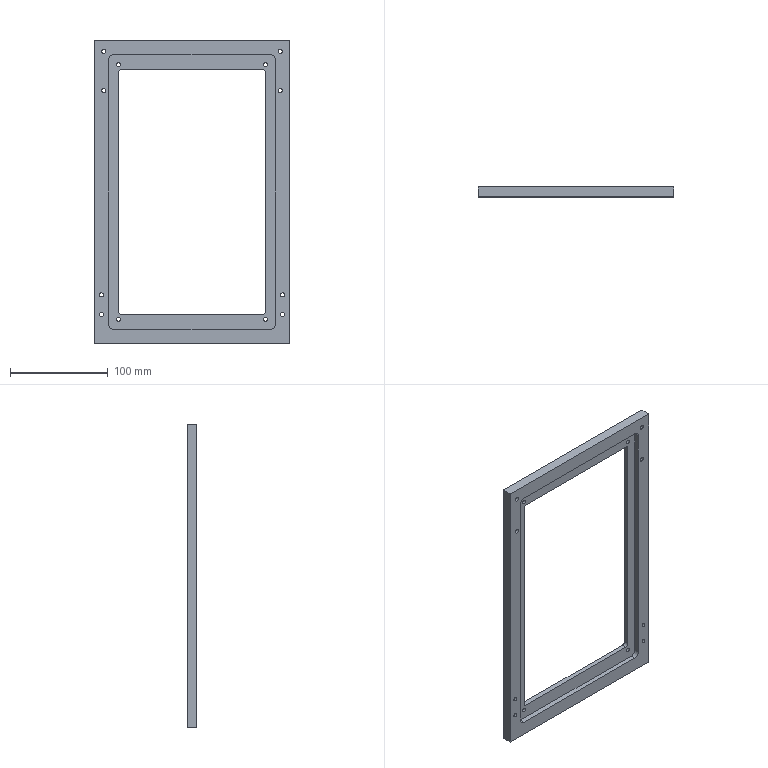Part | SolidWorks | features HoleWzd 3, Cut 2, Fillet 2, Extrusion 1 | 1 solid | 47 faces | box 200 x 10 x 310 mm | volume 193260 mm3 | cylinder 32 | plane 15 | commonest cylinder face diameters 4.2 x24 6 x4 10 x4
STEP:
#1=CARTESIAN_POINT('',(-75.,5.,132.1));
#2=VERTEX_POINT('',#1);
#3=CARTESIAN_POINT('',(-75.,5.,127.9));
#4=VERTEX_POINT('',#3);
#5=CARTESIAN_POINT('',(-75.,5.,130.));
#6=DIRECTION('',(0.,-1.,0.));
#7=DIRECTION('',(0.,0.,-1.));
#8=AXIS2_PLACEMENT_3D('',#5,#6,#7);
#9=CIRCLE('',#8,2.1);
#10=EDGE_CURVE('',#2,#4,#9,.T.);
#11=ORIENTED_EDGE('',*,*,#10,.F.);
#12=CARTESIAN_POINT('',(-75.,0.,132.1));
#13=VERTEX_POINT('',#12);
#14=CARTESIAN_POINT('',(-75.,0.,132.1));
#15=DIRECTION('',(0.,-1.,0.));
#16=VECTOR('',#15,1000.);
#17=LINE('',#14,#16);
#18=EDGE_CURVE('',#2,#13,#17,.T.);
#19=ORIENTED_EDGE('',*,*,#18,.T.);
#20=CARTESIAN_POINT('',(-75.,0.,127.9));
#21=VERTEX_POINT('',#20);
#22=CARTESIAN_POINT('',(-75.,0.,130.));
#23=DIRECTION('',(0.,-1.,0.));
#24=DIRECTION('',(0.,0.,-1.));
#25=AXIS2_PLACEMENT_3D('',#22,#23,#24);
#26=CIRCLE('',#25,2.1);
#27=EDGE_CURVE('',#13,#21,#26,.T.);
#28=ORIENTED_EDGE('',*,*,#27,.T.);
#29=CARTESIAN_POINT('',(-75.,0.,127.9));
#30=DIRECTION('',(0.,-1.,0.));
#31=VECTOR('',#30,1000.);
#32=LINE('',#29,#31);
#33=EDGE_CURVE('',#4,#21,#32,.T.);
#34=ORIENTED_EDGE('',*,*,#33,.F.);
#35=EDGE_LOOP('',(#11,#19,#28,#34));
#36=FACE_OUTER_BOUND('',#35,.T.);
#37=CARTESIAN_POINT('',(-75.,0.,130.));
#38=DIRECTION('',(0.,-1.,0.));
#39=DIRECTION('',(0.,0.,-1.));
#40=AXIS2_PLACEMENT_3D('',#37,#38,#39);
#41=CYLINDRICAL_SURFACE('',#40,2.1);
#42=ADVANCED_FACE('',(#36),#41,.F.);
#43=CARTESIAN_POINT('',(75.,5.,132.1));
#44=VERTEX_POINT('',#43);
#45=CARTESIAN_POINT('',(75.,5.,127.9));
#46=VERTEX_POINT('',#45);
#47=CARTESIAN_POINT('',(75.,5.,130.));
#48=DIRECTION('',(0.,-1.,0.));
#49=DIRECTION('',(0.,0.,-1.));
#50=AXIS2_PLACEMENT_3D('',#47,#48,#49);
#51=CIRCLE('',#50,2.1);
#52=EDGE_CURVE('',#44,#46,#51,.T.);
#53=ORIENTED_EDGE('',*,*,#52,.F.);
#54=CARTESIAN_POINT('',(75.,0.,132.1));
#55=VERTEX_POINT('',#54);
#56=CARTESIAN_POINT('',(75.,0.,132.1));
#57=DIRECTION('',(0.,-1.,0.));
#58=VECTOR('',#57,1000.);
#59=LINE('',#56,#58);
#60=EDGE_CURVE('',#44,#55,#59,.T.);
#61=ORIENTED_EDGE('',*,*,#60,.T.);
#62=CARTESIAN_POINT('',(75.,0.,127.9));
#63=VERTEX_POINT('',#62);
#64=CARTESIAN_POINT('',(75.,0.,130.));
#65=DIRECTION('',(0.,-1.,0.));
#66=DIRECTION('',(0.,0.,-1.));
#67=AXIS2_PLACEMENT_3D('',#64,#65,#66);
#68=CIRCLE('',#67,2.1);
#69=EDGE_CURVE('',#55,#63,#68,.T.);
#70=ORIENTED_EDGE('',*,*,#69,.T.);
#71=CARTESIAN_POINT('',(75.,0.,127.9));
#72=DIRECTION('',(0.,-1.,0.));
#73=VECTOR('',#72,1000.);
#74=LINE('',#71,#73);
#75=EDGE_CURVE('',#46,#63,#74,.T.);
#76=ORIENTED_EDGE('',*,*,#75,.F.);
#77=EDGE_LOOP('',(#53,#61,#70,#76));
#78=FACE_OUTER_BOUND('',#77,.T.);
#79=CARTESIAN_POINT('',(75.,0.,130.));
#80=DIRECTION('',(0.,-1.,0.));
#81=DIRECTION('',(0.,0.,-1.));
#82=AXIS2_PLACEMENT_3D('',#79,#80,#81);
#83=CYLINDRICAL_SURFACE('',#82,2.1);
#84=ADVANCED_FACE('',(#78),#83,.F.);
#85=CARTESIAN_POINT('',(-75.,5.,-127.9));
#86=VERTEX_POINT('',#85);
#87=CARTESIAN_POINT('',(-75.,5.,-132.1));
#88=VERTEX_POINT('',#87);
#89=CARTESIAN_POINT('',(-75.,5.,-130.));
#90=DIRECTION('',(0.,-1.,0.));
#91=DIRECTION('',(0.,0.,-1.));
#92=AXIS2_PLACEMENT_3D('',#89,#90,#91);
#93=CIRCLE('',#92,2.1);
#94=EDGE_CURVE('',#86,#88,#93,.T.);
#95=ORIENTED_EDGE('',*,*,#94,.F.);
#96=CARTESIAN_POINT('',(-75.,0.,-127.9));
#97=VERTEX_POINT('',#96);
#98=CARTESIAN_POINT('',(-75.,0.,-127.9));
#99=DIRECTION('',(0.,-1.,0.));
#100=VECTOR('',#99,1000.);
#101=LINE('',#98,#100);
#102=EDGE_CURVE('',#86,#97,#101,.T.);
#103=ORIENTED_EDGE('',*,*,#102,.T.);
#104=CARTESIAN_POINT('',(-75.,0.,-132.1));
#105=VERTEX_POINT('',#104);
#106=CARTESIAN_POINT('',(-75.,0.,-130.));
#107=DIRECTION('',(0.,-1.,0.));
#108=DIRECTION('',(0.,0.,-1.));
#109=AXIS2_PLACEMENT_3D('',#106,#107,#108);
#110=CIRCLE('',#109,2.1);
#111=EDGE_CURVE('',#97,#105,#110,.T.);
#112=ORIENTED_EDGE('',*,*,#111,.T.);
#113=CARTESIAN_POINT('',(-75.,0.,-132.1));
#114=DIRECTION('',(0.,-1.,0.));
#115=VECTOR('',#114,1000.);
#116=LINE('',#113,#115);
#117=EDGE_CURVE('',#88,#105,#116,.T.);
#118=ORIENTED_EDGE('',*,*,#117,.F.);
#119=EDGE_LOOP('',(#95,#103,#112,#118));
#120=FACE_OUTER_BOUND('',#119,.T.);
#121=CARTESIAN_POINT('',(-75.,0.,-130.));
#122=DIRECTION('',(0.,-1.,0.));
#123=DIRECTION('',(0.,0.,-1.));
#124=AXIS2_PLACEMENT_3D('',#121,#122,#123);
#125=CYLINDRICAL_SURFACE('',#124,2.1);
#126=ADVANCED_FACE('',(#120),#125,.F.);
#127=CARTESIAN_POINT('',(75.,5.,-127.9));
#128=VERTEX_POINT('',#127);
#129=CARTESIAN_POINT('',(75.,5.,-132.1));
#130=VERTEX_POINT('',#129);
#131=CARTESIAN_POINT('',(75.,5.,-130.));
#132=DIRECTION('',(0.,-1.,0.));
#133=DIRECTION('',(0.,0.,-1.));
#134=AXIS2_PLACEMENT_3D('',#131,#132,#133);
#135=CIRCLE('',#134,2.1);
#136=EDGE_CURVE('',#128,#130,#135,.T.);
#137=ORIENTED_EDGE('',*,*,#136,.F.);
#138=CARTESIAN_POINT('',(75.,0.,-127.9));
#139=VERTEX_POINT('',#138);
#140=CARTESIAN_POINT('',(75.,0.,-127.9));
#141=DIRECTION('',(0.,-1.,0.));
#142=VECTOR('',#141,1000.);
#143=LINE('',#140,#142);
#144=EDGE_CURVE('',#128,#139,#143,.T.);
#145=ORIENTED_EDGE('',*,*,#144,.T.);
#146=CARTESIAN_POINT('',(75.,0.,-132.1));
#147=VERTEX_POINT('',#146);
#148=CARTESIAN_POINT('',(75.,0.,-130.));
#149=DIRECTION('',(0.,-1.,0.));
#150=DIRECTION('',(0.,0.,-1.));
#151=AXIS2_PLACEMENT_3D('',#148,#149,#150);
#152=CIRCLE('',#151,2.1);
#153=EDGE_CURVE('',#139,#147,#152,.T.);
#154=ORIENTED_EDGE('',*,*,#153,.T.);
#155=CARTESIAN_POINT('',(75.,0.,-132.1));
#156=DIRECTION('',(0.,-1.,0.));
#157=VECTOR('',#156,1000.);
#158=LINE('',#155,#157);
#159=EDGE_CURVE('',#130,#147,#158,.T.);
#160=ORIENTED_EDGE('',*,*,#159,.F.);
#161=EDGE_LOOP('',(#137,#145,#154,#160));
#162=FACE_OUTER_BOUND('',#161,.T.);
#163=CARTESIAN_POINT('',(75.,0.,-130.));
#164=DIRECTION('',(0.,-1.,0.));
#165=DIRECTION('',(0.,0.,-1.));
#166=AXIS2_PLACEMENT_3D('',#163,#164,#165);
#167=CYLINDRICAL_SURFACE('',#166,2.1);
#168=ADVANCED_FACE('',(#162),#167,.F.);
#169=CARTESIAN_POINT('',(-90.,-5.,101.4));
#170=VERTEX_POINT('',#169);
#171=CARTESIAN_POINT('',(-90.,-5.,105.6));
#172=VERTEX_POINT('',#171);
#173=CARTESIAN_POINT('',(-90.,-5.,103.5));
#174=DIRECTION('',(0.,1.,0.));
#175=DIRECTION('',(0.,0.,1.));
#176=AXIS2_PLACEMENT_3D('',#173,#174,#175);
#177=CIRCLE('',#176,2.1);
#178=EDGE_CURVE('',#170,#172,#177,.T.);
#179=ORIENTED_EDGE('',*,*,#178,.F.);
#180=CARTESIAN_POINT('',(-90.,5.,101.4));
#181=VERTEX_POINT('',#180);
#182=CARTESIAN_POINT('',(-90.,5.,101.4));
#183=DIRECTION('',(0.,1.,0.));
#184=VECTOR('',#183,1000.);
#185=LINE('',#182,#184);
#186=EDGE_CURVE('',#170,#181,#185,.T.);
#187=ORIENTED_EDGE('',*,*,#186,.T.);
#188=CARTESIAN_POINT('',(-90.,5.,105.6));
#189=VERTEX_POINT('',#188);
#190=CARTESIAN_POINT('',(-90.,5.,103.5));
#191=DIRECTION('',(0.,1.,0.));
#192=DIRECTION('',(0.,0.,1.));
#193=AXIS2_PLACEMENT_3D('',#190,#191,#192);
#194=CIRCLE('',#193,2.1);
#195=EDGE_CURVE('',#181,#189,#194,.T.);
#196=ORIENTED_EDGE('',*,*,#195,.T.);
#197=CARTESIAN_POINT('',(-90.,5.,105.6));
#198=DIRECTION('',(0.,1.,0.));
#199=VECTOR('',#198,1000.);
#200=LINE('',#197,#199);
#201=EDGE_CURVE('',#172,#189,#200,.T.);
#202=ORIENTED_EDGE('',*,*,#201,.F.);
#203=EDGE_LOOP('',(#179,#187,#196,#202));
#204=FACE_OUTER_BOUND('',#203,.T.);
#205=CARTESIAN_POINT('',(-90.,5.,103.5));
#206=DIRECTION('',(0.,1.,0.));
#207=DIRECTION('',(0.,0.,1.));
#208=AXIS2_PLACEMENT_3D('',#205,#206,#207);
#209=CYLINDRICAL_SURFACE('',#208,2.1);
#210=ADVANCED_FACE('',(#204),#209,.F.);
#211=CARTESIAN_POINT('',(-90.,-5.,141.4));
#212=VERTEX_POINT('',#211);
#213=CARTESIAN_POINT('',(-90.,-5.,145.6));
#214=VERTEX_POINT('',#213);
#215=CARTESIAN_POINT('',(-90.,-5.,143.5));
#216=DIRECTION('',(0.,1.,0.));
#217=DIRECTION('',(0.,0.,1.));
#218=AXIS2_PLACEMENT_3D('',#215,#216,#217);
#219=CIRCLE('',#218,2.1);
#220=EDGE_CURVE('',#212,#214,#219,.T.);
#221=ORIENTED_EDGE('',*,*,#220,.F.);
#222=CARTESIAN_POINT('',(-90.,5.,141.4));
#223=VERTEX_POINT('',#222);
#224=CARTESIAN_POINT('',(-90.,5.,141.4));
#225=DIRECTION('',(0.,1.,0.));
#226=VECTOR('',#225,1000.);
#227=LINE('',#224,#226);
#228=EDGE_CURVE('',#212,#223,#227,.T.);
#229=ORIENTED_EDGE('',*,*,#228,.T.);
#230=CARTESIAN_POINT('',(-90.,5.,145.6));
#231=VERTEX_POINT('',#230);
#232=CARTESIAN_POINT('',(-90.,5.,143.5));
#233=DIRECTION('',(0.,1.,0.));
#234=DIRECTION('',(0.,0.,1.));
#235=AXIS2_PLACEMENT_3D('',#232,#233,#234);
#236=CIRCLE('',#235,2.1);
#237=EDGE_CURVE('',#223,#231,#236,.T.);
#238=ORIENTED_EDGE('',*,*,#237,.T.);
#239=CARTESIAN_POINT('',(-90.,5.,145.6));
#240=DIRECTION('',(0.,1.,0.));
#241=VECTOR('',#240,1000.);
#242=LINE('',#239,#241);
#243=EDGE_CURVE('',#214,#231,#242,.T.);
#244=ORIENTED_EDGE('',*,*,#243,.F.);
#245=EDGE_LOOP('',(#221,#229,#238,#244));
#246=FACE_OUTER_BOUND('',#245,.T.);
#247=CARTESIAN_POINT('',(-90.,5.,143.5));
#248=DIRECTION('',(0.,1.,0.));
#249=DIRECTION('',(0.,0.,1.));
#250=AXIS2_PLACEMENT_3D('',#247,#248,#249);
#251=CYLINDRICAL_SURFACE('',#250,2.1);
#252=ADVANCED_FACE('',(#246),#251,.F.);
#253=CARTESIAN_POINT('',(90.,-5.,101.4));
#254=VERTEX_POINT('',#253);
#255=CARTESIAN_POINT('',(90.,-5.,105.6));
#256=VERTEX_POINT('',#255);
#257=CARTESIAN_POINT('',(90.,-5.,103.5));
#258=DIRECTION('',(0.,1.,0.));
#259=DIRECTION('',(0.,0.,1.));
#260=AXIS2_PLACEMENT_3D('',#257,#258,#259);
#261=CIRCLE('',#260,2.1);
#262=EDGE_CURVE('',#254,#256,#261,.T.);
#263=ORIENTED_EDGE('',*,*,#262,.F.);
#264=CARTESIAN_POINT('',(90.,5.,101.4));
#265=VERTEX_POINT('',#264);
#266=CARTESIAN_POINT('',(90.,5.,101.4));
#267=DIRECTION('',(0.,1.,0.));
#268=VECTOR('',#267,1000.);
#269=LINE('',#266,#268);
#270=EDGE_CURVE('',#254,#265,#269,.T.);
#271=ORIENTED_EDGE('',*,*,#270,.T.);
#272=CARTESIAN_POINT('',(90.,5.,105.6));
#273=VERTEX_POINT('',#272);
#274=CARTESIAN_POINT('',(90.,5.,103.5));
#275=DIRECTION('',(0.,1.,0.));
#276=DIRECTION('',(0.,0.,1.));
#277=AXIS2_PLACEMENT_3D('',#274,#275,#276);
#278=CIRCLE('',#277,2.1);
#279=EDGE_CURVE('',#265,#273,#278,.T.);
#280=ORIENTED_EDGE('',*,*,#279,.T.);
#281=CARTESIAN_POINT('',(90.,5.,105.6));
#282=DIRECTION('',(0.,1.,0.));
#283=VECTOR('',#282,1000.);
#284=LINE('',#281,#283);
#285=EDGE_CURVE('',#256,#273,#284,.T.);
#286=ORIENTED_EDGE('',*,*,#285,.F.);
#287=EDGE_LOOP('',(#263,#271,#280,#286));
#288=FACE_OUTER_BOUND('',#287,.T.);
#289=CARTESIAN_POINT('',(90.,5.,103.5));
#290=DIRECTION('',(0.,1.,0.));
#291=DIRECTION('',(0.,0.,1.));
#292=AXIS2_PLACEMENT_3D('',#289,#290,#291);
#293=CYLINDRICAL_SURFACE('',#292,2.1);
#294=ADVANCED_FACE('',(#288),#293,.F.);
#295=CARTESIAN_POINT('',(90.,-5.,141.4));
#296=VERTEX_POINT('',#295);
#297=CARTESIAN_POINT('',(90.,-5.,145.6));
#298=VERTEX_POINT('',#297);
#299=CARTESIAN_POINT('',(90.,-5.,143.5));
#300=DIRECTION('',(0.,1.,0.));
#301=DIRECTION('',(0.,0.,1.));
#302=AXIS2_PLACEMENT_3D('',#299,#300,#301);
#303=CIRCLE('',#302,2.1);
#304=EDGE_CURVE('',#296,#298,#303,.T.);
#305=ORIENTED_EDGE('',*,*,#304,.F.);
#306=CARTESIAN_POINT('',(90.,5.,141.4));
#307=VERTEX_POINT('',#306);
#308=CARTESIAN_POINT('',(90.,5.,141.4));
#309=DIRECTION('',(0.,1.,0.));
#310=VECTOR('',#309,1000.);
#311=LINE('',#308,#310);
#312=EDGE_CURVE('',#296,#307,#311,.T.);
#313=ORIENTED_EDGE('',*,*,#312,.T.);
#314=CARTESIAN_POINT('',(90.,5.,145.6));
#315=VERTEX_POINT('',#314);
#316=CARTESIAN_POINT('',(90.,5.,143.5));
#317=DIRECTION('',(0.,1.,0.));
#318=DIRECTION('',(0.,0.,1.));
#319=AXIS2_PLACEMENT_3D('',#316,#317,#318);
#320=CIRCLE('',#319,2.1);
#321=EDGE_CURVE('',#307,#315,#320,.T.);
#322=ORIENTED_EDGE('',*,*,#321,.T.);
#323=CARTESIAN_POINT('',(90.,5.,145.6));
#324=DIRECTION('',(0.,1.,0.));
#325=VECTOR('',#324,1000.);
#326=LINE('',#323,#325);
#327=EDGE_CURVE('',#298,#315,#326,.T.);
#328=ORIENTED_EDGE('',*,*,#327,.F.);
#329=EDGE_LOOP('',(#305,#313,#322,#328));
#330=FACE_OUTER_BOUND('',#329,.T.);
#331=CARTESIAN_POINT('',(90.,5.,143.5));
#332=DIRECTION('',(0.,1.,0.));
#333=DIRECTION('',(0.,0.,1.));
#334=AXIS2_PLACEMENT_3D('',#331,#332,#333);
#335=CYLINDRICAL_SURFACE('',#334,2.1);
#336=ADVANCED_FACE('',(#330),#335,.F.);
#337=CARTESIAN_POINT('',(92.5,-5.,-107.1));
#338=VERTEX_POINT('',#337);
#339=CARTESIAN_POINT('',(92.5,-5.,-102.9));
#340=VERTEX_POINT('',#339);
#341=CARTESIAN_POINT('',(92.5,-5.,-105.));
#342=DIRECTION('',(0.,1.,0.));
#343=DIRECTION('',(0.,0.,1.));
#344=AXIS2_PLACEMENT_3D('',#341,#342,#343);
#345=CIRCLE('',#344,2.1);
#346=EDGE_CURVE('',#338,#340,#345,.T.);
#347=ORIENTED_EDGE('',*,*,#346,.F.);
#348=CARTESIAN_POINT('',(92.5,5.,-107.1));
#349=VERTEX_POINT('',#348);
#350=CARTESIAN_POINT('',(92.5,5.,-107.1));
#351=DIRECTION('',(0.,1.,0.));
#352=VECTOR('',#351,1000.);
#353=LINE('',#350,#352);
#354=EDGE_CURVE('',#338,#349,#353,.T.);
#355=ORIENTED_EDGE('',*,*,#354,.T.);
#356=CARTESIAN_POINT('',(92.5,5.,-102.9));
#357=VERTEX_POINT('',#356);
#358=CARTESIAN_POINT('',(92.5,5.,-105.));
#359=DIRECTION('',(0.,1.,0.));
#360=DIRECTION('',(0.,0.,1.));
#361=AXIS2_PLACEMENT_3D('',#358,#359,#360);
#362=CIRCLE('',#361,2.1);
#363=EDGE_CURVE('',#349,#357,#362,.T.);
#364=ORIENTED_EDGE('',*,*,#363,.T.);
#365=CARTESIAN_POINT('',(92.5,5.,-102.9));
#366=DIRECTION('',(0.,1.,0.));
#367=VECTOR('',#366,1000.);
#368=LINE('',#365,#367);
#369=EDGE_CURVE('',#340,#357,#368,.T.);
#370=ORIENTED_EDGE('',*,*,#369,.F.);
#371=EDGE_LOOP('',(#347,#355,#364,#370));
#372=FACE_OUTER_BOUND('',#371,.T.);
#373=CARTESIAN_POINT('',(92.5,5.,-105.));
#374=DIRECTION('',(0.,1.,0.));
#375=DIRECTION('',(0.,0.,1.));
#376=AXIS2_PLACEMENT_3D('',#373,#374,#375);
#377=CYLINDRICAL_SURFACE('',#376,2.1);
#378=ADVANCED_FACE('',(#372),#377,.F.);
#379=CARTESIAN_POINT('',(92.5,-5.,-127.1));
#380=VERTEX_POINT('',#379);
#381=CARTESIAN_POINT('',(92.5,-5.,-122.9));
#382=VERTEX_POINT('',#381);
#383=CARTESIAN_POINT('',(92.5,-5.,-125.));
#384=DIRECTION('',(0.,1.,0.));
#385=DIRECTION('',(0.,0.,1.));
#386=AXIS2_PLACEMENT_3D('',#383,#384,#385);
#387=CIRCLE('',#386,2.1);
#388=EDGE_CURVE('',#380,#382,#387,.T.);
#389=ORIENTED_EDGE('',*,*,#388,.F.);
#390=CARTESIAN_POINT('',(92.5,5.,-127.1));
#391=VERTEX_POINT('',#390);
#392=CARTESIAN_POINT('',(92.5,5.,-127.1));
#393=DIRECTION('',(0.,1.,0.));
#394=VECTOR('',#393,1000.);
#395=LINE('',#392,#394);
#396=EDGE_CURVE('',#380,#391,#395,.T.);
#397=ORIENTED_EDGE('',*,*,#396,.T.);
#398=CARTESIAN_POINT('',(92.5,5.,-122.9));
#399=VERTEX_POINT('',#398);
#400=CARTESIAN_POINT('',(92.5,5.,-125.));
#401=DIRECTION('',(0.,1.,0.));
#402=DIRECTION('',(0.,0.,1.));
#403=AXIS2_PLACEMENT_3D('',#400,#401,#402);
#404=CIRCLE('',#403,2.1);
#405=EDGE_CURVE('',#391,#399,#404,.T.);
#406=ORIENTED_EDGE('',*,*,#405,.T.);
#407=CARTESIAN_POINT('',(92.5,5.,-122.9));
#408=DIRECTION('',(0.,1.,0.));
#409=VECTOR('',#408,1000.);
#410=LINE('',#407,#409);
#411=EDGE_CURVE('',#382,#399,#410,.T.);
#412=ORIENTED_EDGE('',*,*,#411,.F.);
#413=EDGE_LOOP('',(#389,#397,#406,#412));
#414=FACE_OUTER_BOUND('',#413,.T.);
#415=CARTESIAN_POINT('',(92.5,5.,-125.));
#416=DIRECTION('',(0.,1.,0.));
#417=DIRECTION('',(0.,0.,1.));
#418=AXIS2_PLACEMENT_3D('',#415,#416,#417);
#419=CYLINDRICAL_SURFACE('',#418,2.1);
#420=ADVANCED_FACE('',(#414),#419,.F.);
#421=CARTESIAN_POINT('',(-92.5,-5.,-107.1));
#422=VERTEX_POINT('',#421);
#423=CARTESIAN_POINT('',(-92.5,-5.,-102.9));
#424=VERTEX_POINT('',#423);
#425=CARTESIAN_POINT('',(-92.5,-5.,-105.));
#426=DIRECTION('',(0.,1.,0.));
#427=DIRECTION('',(0.,0.,1.));
#428=AXIS2_PLACEMENT_3D('',#425,#426,#427);
#429=CIRCLE('',#428,2.1);
#430=EDGE_CURVE('',#422,#424,#429,.T.);
#431=ORIENTED_EDGE('',*,*,#430,.F.);
#432=CARTESIAN_POINT('',(-92.5,5.,-107.1));
#433=VERTEX_POINT('',#432);
#434=CARTESIAN_POINT('',(-92.5,5.,-107.1));
#435=DIRECTION('',(0.,1.,0.));
#436=VECTOR('',#435,1000.);
#437=LINE('',#434,#436);
#438=EDGE_CURVE('',#422,#433,#437,.T.);
#439=ORIENTED_EDGE('',*,*,#438,.T.);
#440=CARTESIAN_POINT('',(-92.5,5.,-102.9));
#441=VERTEX_POINT('',#440);
#442=CARTESIAN_POINT('',(-92.5,5.,-105.));
#443=DIRECTION('',(0.,1.,0.));
#444=DIRECTION('',(0.,0.,1.));
#445=AXIS2_PLACEMENT_3D('',#442,#443,#444);
#446=CIRCLE('',#445,2.1);
#447=EDGE_CURVE('',#433,#441,#446,.T.);
#448=ORIENTED_EDGE('',*,*,#447,.T.);
#449=CARTESIAN_POINT('',(-92.5,5.,-102.9));
#450=DIRECTION('',(0.,1.,0.));
#451=VECTOR('',#450,1000.);
#452=LINE('',#449,#451);
#453=EDGE_CURVE('',#424,#441,#452,.T.);
#454=ORIENTED_EDGE('',*,*,#453,.F.);
#455=EDGE_LOOP('',(#431,#439,#448,#454));
#456=FACE_OUTER_BOUND('',#455,.T.);
#457=CARTESIAN_POINT('',(-92.5,5.,-105.));
#458=DIRECTION('',(0.,1.,0.));
#459=DIRECTION('',(0.,0.,1.));
#460=AXIS2_PLACEMENT_3D('',#457,#458,#459);
#461=CYLINDRICAL_SURFACE('',#460,2.1);
#462=ADVANCED_FACE('',(#456),#461,.F.);
#463=CARTESIAN_POINT('',(-92.5,-5.,-127.1));
#464=VERTEX_POINT('',#463);
#465=CARTESIAN_POINT('',(-92.5,-5.,-122.9));
#466=VERTEX_POINT('',#465);
#467=CARTESIAN_POINT('',(-92.5,-5.,-125.));
#468=DIRECTION('',(0.,1.,0.));
#469=DIRECTION('',(0.,0.,1.));
#470=AXIS2_PLACEMENT_3D('',#467,#468,#469);
#471=CIRCLE('',#470,2.1);
#472=EDGE_CURVE('',#464,#466,#471,.T.);
#473=ORIENTED_EDGE('',*,*,#472,.F.);
#474=CARTESIAN_POINT('',(-92.5,5.,-127.1));
#475=VERTEX_POINT('',#474);
#476=CARTESIAN_POINT('',(-92.5,5.,-127.1));
#477=DIRECTION('',(0.,1.,0.));
#478=VECTOR('',#477,1000.);
#479=LINE('',#476,#478);
#480=EDGE_CURVE('',#464,#475,#479,.T.);
#481=ORIENTED_EDGE('',*,*,#480,.T.);
#482=CARTESIAN_POINT('',(-92.5,5.,-122.9));
#483=VERTEX_POINT('',#482);
#484=CARTESIAN_POINT('',(-92.5,5.,-125.));
#485=DIRECTION('',(0.,1.,0.));
#486=DIRECTION('',(0.,0.,1.));
#487=AXIS2_PLACEMENT_3D('',#484,#485,#486);
#488=CIRCLE('',#487,2.1);
#489=EDGE_CURVE('',#475,#483,#488,.T.);
#490=ORIENTED_EDGE('',*,*,#489,.T.);
#491=CARTESIAN_POINT('',(-92.5,5.,-122.9));
#492=DIRECTION('',(0.,1.,0.));
#493=VECTOR('',#492,1000.);
#494=LINE('',#491,#493);
#495=EDGE_CURVE('',#466,#483,#494,.T.);
#496=ORIENTED_EDGE('',*,*,#495,.F.);
#497=EDGE_LOOP('',(#473,#481,#490,#496));
#498=FACE_OUTER_BOUND('',#497,.T.);
#499=CARTESIAN_POINT('',(-92.5,5.,-125.));
#500=DIRECTION('',(0.,1.,0.));
#501=DIRECTION('',(0.,0.,1.));
#502=AXIS2_PLACEMENT_3D('',#499,#500,#501);
#503=CYLINDRICAL_SURFACE('',#502,2.1);
#504=ADVANCED_FACE('',(#498),#503,.F.);
#505=CARTESIAN_POINT('',(75.,0.,122.));
#506=VERTEX_POINT('',#505);
#507=CARTESIAN_POINT('',(75.,0.,-122.));
#508=VERTEX_POINT('',#507);
#509=CARTESIAN_POINT('',(75.,0.,-125.));
#510=DIRECTION('',(0.,0.,-1.));
#511=VECTOR('',#510,1000.);
#512=LINE('',#509,#511);
#513=EDGE_CURVE('',#506,#508,#512,.T.);
#514=ORIENTED_EDGE('',*,*,#513,.F.);
#515=CARTESIAN_POINT('',(75.,5.,122.));
#516=VERTEX_POINT('',#515);
#517=CARTESIAN_POINT('',(75.,5.,122.));
#518=DIRECTION('',(0.,1.,0.));
#519=VECTOR('',#518,1000.);
#520=LINE('',#517,#519);
#521=EDGE_CURVE('',#506,#516,#520,.T.);
#522=ORIENTED_EDGE('',*,*,#521,.T.);
#523=CARTESIAN_POINT('',(75.,5.,-122.));
#524=VERTEX_POINT('',#523);
#525=CARTESIAN_POINT('',(75.,5.,-125.));
#526=DIRECTION('',(0.,0.,1.));
#527=VECTOR('',#526,1000.);
#528=LINE('',#525,#527);
#529=EDGE_CURVE('',#524,#516,#528,.T.);
#530=ORIENTED_EDGE('',*,*,#529,.F.);
#531=CARTESIAN_POINT('',(75.,-5.,-122.));
#532=DIRECTION('',(0.,-1.,0.));
#533=VECTOR('',#532,1000.);
#534=LINE('',#531,#533);
#535=EDGE_CURVE('',#524,#508,#534,.T.);
#536=ORIENTED_EDGE('',*,*,#535,.T.);
#537=EDGE_LOOP('',(#514,#522,#530,#536));
#538=FACE_OUTER_BOUND('',#537,.T.);
#539=CARTESIAN_POINT('',(75.,5.,-125.));
#540=DIRECTION('',(1.,0.,0.));
#541=DIRECTION('',(0.,0.,-1.));
#542=AXIS2_PLACEMENT_3D('',#539,#540,#541);
#543=PLANE('',#542);
#544=ADVANCED_FACE('',(#538),#543,.F.);
#545=CARTESIAN_POINT('',(72.,0.,-125.));
#546=VERTEX_POINT('',#545);
#547=CARTESIAN_POINT('',(-72.,0.,-125.));
#548=VERTEX_POINT('',#547);
#549=CARTESIAN_POINT('',(-75.,0.,-125.));
#550=DIRECTION('',(-1.,0.,0.));
#551=VECTOR('',#550,1000.);
#552=LINE('',#549,#551);
#553=EDGE_CURVE('',#546,#548,#552,.T.);
#554=ORIENTED_EDGE('',*,*,#553,.F.);
#555=CARTESIAN_POINT('',(72.,5.,-125.));
#556=VERTEX_POINT('',#555);
#557=CARTESIAN_POINT('',(72.,5.,-125.));
#558=DIRECTION('',(0.,1.,0.));
#559=VECTOR('',#558,1000.);
#560=LINE('',#557,#559);
#561=EDGE_CURVE('',#546,#556,#560,.T.);
#562=ORIENTED_EDGE('',*,*,#561,.T.);
#563=CARTESIAN_POINT('',(-72.,5.,-125.));
#564=VERTEX_POINT('',#563);
#565=CARTESIAN_POINT('',(-75.,5.,-125.));
#566=DIRECTION('',(1.,0.,0.));
#567=VECTOR('',#566,1000.);
#568=LINE('',#565,#567);
#569=EDGE_CURVE('',#564,#556,#568,.T.);
#570=ORIENTED_EDGE('',*,*,#569,.F.);
#571=CARTESIAN_POINT('',(-72.,-5.,-125.));
#572=DIRECTION('',(0.,-1.,0.));
#573=VECTOR('',#572,1000.);
#574=LINE('',#571,#573);
#575=EDGE_CURVE('',#564,#548,#574,.T.);
#576=ORIENTED_EDGE('',*,*,#575,.T.);
#577=EDGE_LOOP('',(#554,#562,#570,#576));
#578=FACE_OUTER_BOUND('',#577,.T.);
#579=CARTESIAN_POINT('',(-75.,5.,-125.));
#580=DIRECTION('',(0.,0.,-1.));
#581=DIRECTION('',(-1.,0.,0.));
#582=AXIS2_PLACEMENT_3D('',#579,#580,#581);
#583=PLANE('',#582);
#584=ADVANCED_FACE('',(#578),#583,.F.);
#585=CARTESIAN_POINT('',(-75.,0.,-122.));
#586=VERTEX_POINT('',#585);
#587=CARTESIAN_POINT('',(-75.,0.,122.));
#588=VERTEX_POINT('',#587);
#589=CARTESIAN_POINT('',(-75.,0.,-125.));
#590=DIRECTION('',(0.,0.,1.));
#591=VECTOR('',#590,1000.);
#592=LINE('',#589,#591);
#593=EDGE_CURVE('',#586,#588,#592,.T.);
#594=ORIENTED_EDGE('',*,*,#593,.F.);
#595=CARTESIAN_POINT('',(-75.,5.,-122.));
#596=VERTEX_POINT('',#595);
#597=CARTESIAN_POINT('',(-75.,5.,-122.));
#598=DIRECTION('',(0.,1.,0.));
#599=VECTOR('',#598,1000.);
#600=LINE('',#597,#599);
#601=EDGE_CURVE('',#586,#596,#600,.T.);
#602=ORIENTED_EDGE('',*,*,#601,.T.);
#603=CARTESIAN_POINT('',(-75.,5.,122.));
#604=VERTEX_POINT('',#603);
#605=CARTESIAN_POINT('',(-75.,5.,-125.));
#606=DIRECTION('',(0.,0.,-1.));
#607=VECTOR('',#606,1000.);
#608=LINE('',#605,#607);
#609=EDGE_CURVE('',#604,#596,#608,.T.);
#610=ORIENTED_EDGE('',*,*,#609,.F.);
#611=CARTESIAN_POINT('',(-75.,-5.,122.));
#612=DIRECTION('',(0.,-1.,0.));
#613=VECTOR('',#612,1000.);
#614=LINE('',#611,#613);
#615=EDGE_CURVE('',#604,#588,#614,.T.);
#616=ORIENTED_EDGE('',*,*,#615,.T.);
#617=EDGE_LOOP('',(#594,#602,#610,#616));
#618=FACE_OUTER_BOUND('',#617,.T.);
#619=CARTESIAN_POINT('',(-75.,5.,-125.));
#620=DIRECTION('',(-1.,0.,0.));
#621=DIRECTION('',(0.,0.,1.));
#622=AXIS2_PLACEMENT_3D('',#619,#620,#621);
#623=PLANE('',#622);
#624=ADVANCED_FACE('',(#618),#623,.F.);
#625=CARTESIAN_POINT('',(-72.,0.,125.));
#626=VERTEX_POINT('',#625);
#627=CARTESIAN_POINT('',(72.,0.,125.));
#628=VERTEX_POINT('',#627);
#629=CARTESIAN_POINT('',(-75.,0.,125.));
#630=DIRECTION('',(1.,0.,0.));
#631=VECTOR('',#630,1000.);
#632=LINE('',#629,#631);
#633=EDGE_CURVE('',#626,#628,#632,.T.);
#634=ORIENTED_EDGE('',*,*,#633,.F.);
#635=CARTESIAN_POINT('',(-72.,5.,125.));
#636=VERTEX_POINT('',#635);
#637=CARTESIAN_POINT('',(-72.,5.,125.));
#638=DIRECTION('',(0.,1.,0.));
#639=VECTOR('',#638,1000.);
#640=LINE('',#637,#639);
#641=EDGE_CURVE('',#626,#636,#640,.T.);
#642=ORIENTED_EDGE('',*,*,#641,.T.);
#643=CARTESIAN_POINT('',(72.,5.,125.));
#644=VERTEX_POINT('',#643);
#645=CARTESIAN_POINT('',(-75.,5.,125.));
#646=DIRECTION('',(-1.,0.,0.));
#647=VECTOR('',#646,1000.);
#648=LINE('',#645,#647);
#649=EDGE_CURVE('',#644,#636,#648,.T.);
#650=ORIENTED_EDGE('',*,*,#649,.F.);
#651=CARTESIAN_POINT('',(72.,-5.,125.));
#652=DIRECTION('',(0.,-1.,0.));
#653=VECTOR('',#652,1000.);
#654=LINE('',#651,#653);
#655=EDGE_CURVE('',#644,#628,#654,.T.);
#656=ORIENTED_EDGE('',*,*,#655,.T.);
#657=EDGE_LOOP('',(#634,#642,#650,#656));
#658=FACE_OUTER_BOUND('',#657,.T.);
#659=CARTESIAN_POINT('',(-75.,5.,125.));
#660=DIRECTION('',(0.,0.,1.));
#661=DIRECTION('',(1.,0.,0.));
#662=AXIS2_PLACEMENT_3D('',#659,#660,#661);
#663=PLANE('',#662);
#664=ADVANCED_FACE('',(#658),#663,.F.);
#665=CARTESIAN_POINT('',(-72.,0.,122.));
#666=DIRECTION('',(0.,1.,0.));
#667=DIRECTION('',(0.,0.,-1.));
#668=AXIS2_PLACEMENT_3D('',#665,#666,#667);
#669=CIRCLE('',#668,3.);
#670=EDGE_CURVE('',#588,#626,#669,.T.);
#671=ORIENTED_EDGE('',*,*,#670,.F.);
#672=ORIENTED_EDGE('',*,*,#615,.F.);
#673=CARTESIAN_POINT('',(-72.,5.,122.));
#674=DIRECTION('',(0.,-1.,0.));
#675=DIRECTION('',(0.,0.,1.));
#676=AXIS2_PLACEMENT_3D('',#673,#674,#675);
#677=CIRCLE('',#676,3.);
#678=EDGE_CURVE('',#636,#604,#677,.T.);
#679=ORIENTED_EDGE('',*,*,#678,.F.);
#680=ORIENTED_EDGE('',*,*,#641,.F.);
#681=EDGE_LOOP('',(#671,#672,#679,#680));
#682=FACE_OUTER_BOUND('',#681,.T.);
#683=CARTESIAN_POINT('',(-72.,5.,122.));
#684=DIRECTION('',(0.,1.,0.));
#685=DIRECTION('',(0.,0.,1.));
#686=AXIS2_PLACEMENT_3D('',#683,#684,#685);
#687=CYLINDRICAL_SURFACE('',#686,3.);
#688=ADVANCED_FACE('',(#682),#687,.F.);
#689=CARTESIAN_POINT('',(72.,0.,122.));
#690=DIRECTION('',(0.,1.,0.));
#691=DIRECTION('',(0.,0.,-1.));
#692=AXIS2_PLACEMENT_3D('',#689,#690,#691);
#693=CIRCLE('',#692,3.);
#694=EDGE_CURVE('',#628,#506,#693,.T.);
#695=ORIENTED_EDGE('',*,*,#694,.F.);
#696=ORIENTED_EDGE('',*,*,#655,.F.);
#697=CARTESIAN_POINT('',(72.,5.,122.));
#698=DIRECTION('',(0.,-1.,0.));
#699=DIRECTION('',(0.,0.,1.));
#700=AXIS2_PLACEMENT_3D('',#697,#698,#699);
#701=CIRCLE('',#700,3.);
#702=EDGE_CURVE('',#516,#644,#701,.T.);
#703=ORIENTED_EDGE('',*,*,#702,.F.);
#704=ORIENTED_EDGE('',*,*,#521,.F.);
#705=EDGE_LOOP('',(#695,#696,#703,#704));
#706=FACE_OUTER_BOUND('',#705,.T.);
#707=CARTESIAN_POINT('',(72.,5.,122.));
#708=DIRECTION('',(0.,1.,0.));
#709=DIRECTION('',(0.,0.,1.));
#710=AXIS2_PLACEMENT_3D('',#707,#708,#709);
#711=CYLINDRICAL_SURFACE('',#710,3.);
#712=ADVANCED_FACE('',(#706),#711,.F.);
#713=CARTESIAN_POINT('',(72.,0.,-122.));
#714=DIRECTION('',(0.,1.,0.));
#715=DIRECTION('',(0.,0.,-1.));
#716=AXIS2_PLACEMENT_3D('',#713,#714,#715);
#717=CIRCLE('',#716,3.);
#718=EDGE_CURVE('',#508,#546,#717,.T.);
#719=ORIENTED_EDGE('',*,*,#718,.F.);
#720=ORIENTED_EDGE('',*,*,#535,.F.);
#721=CARTESIAN_POINT('',(72.,5.,-122.));
#722=DIRECTION('',(0.,-1.,0.));
#723=DIRECTION('',(0.,0.,1.));
#724=AXIS2_PLACEMENT_3D('',#721,#722,#723);
#725=CIRCLE('',#724,3.);
#726=EDGE_CURVE('',#556,#524,#725,.T.);
#727=ORIENTED_EDGE('',*,*,#726,.F.);
#728=ORIENTED_EDGE('',*,*,#561,.F.);
#729=EDGE_LOOP('',(#719,#720,#727,#728));
#730=FACE_OUTER_BOUND('',#729,.T.);
#731=CARTESIAN_POINT('',(72.,5.,-122.));
#732=DIRECTION('',(0.,1.,0.));
#733=DIRECTION('',(0.,0.,1.));
#734=AXIS2_PLACEMENT_3D('',#731,#732,#733);
#735=CYLINDRICAL_SURFACE('',#734,3.);
#736=ADVANCED_FACE('',(#730),#735,.F.);
#737=CARTESIAN_POINT('',(-72.,0.,-122.));
#738=DIRECTION('',(0.,1.,0.));
#739=DIRECTION('',(0.,0.,-1.));
#740=AXIS2_PLACEMENT_3D('',#737,#738,#739);
#741=CIRCLE('',#740,3.);
#742=EDGE_CURVE('',#548,#586,#741,.T.);
#743=ORIENTED_EDGE('',*,*,#742,.F.);
#744=ORIENTED_EDGE('',*,*,#575,.F.);
#745=CARTESIAN_POINT('',(-72.,5.,-122.));
#746=DIRECTION('',(0.,-1.,0.));
#747=DIRECTION('',(0.,0.,1.));
#748=AXIS2_PLACEMENT_3D('',#745,#746,#747);
#749=CIRCLE('',#748,3.);
#750=EDGE_CURVE('',#596,#564,#749,.T.);
#751=ORIENTED_EDGE('',*,*,#750,.F.);
#752=ORIENTED_EDGE('',*,*,#601,.F.);
#753=EDGE_LOOP('',(#743,#744,#751,#752));
#754=FACE_OUTER_BOUND('',#753,.T.);
#755=CARTESIAN_POINT('',(-72.,5.,-122.));
#756=DIRECTION('',(0.,1.,0.));
#757=DIRECTION('',(0.,0.,1.));
#758=AXIS2_PLACEMENT_3D('',#755,#756,#757);
#759=CYLINDRICAL_SURFACE('',#758,3.);
#760=ADVANCED_FACE('',(#754),#759,.F.);
#761=CARTESIAN_POINT('',(-100.,-5.,-155.));
#762=VERTEX_POINT('',#761);
#763=CARTESIAN_POINT('',(-100.,-5.,155.));
#764=VERTEX_POINT('',#763);
#765=CARTESIAN_POINT('',(-100.,-5.,155.));
#766=DIRECTION('',(0.,0.,1.));
#767=VECTOR('',#766,1000.);
#768=LINE('',#765,#767);
#769=EDGE_CURVE('',#762,#764,#768,.T.);
#770=ORIENTED_EDGE('',*,*,#769,.T.);
#771=CARTESIAN_POINT('',(-100.,5.,155.));
#772=VERTEX_POINT('',#771);
#773=CARTESIAN_POINT('',(-100.,5.,155.));
#774=DIRECTION('',(0.,-1.,0.));
#775=VECTOR('',#774,1000.);
#776=LINE('',#773,#775);
#777=EDGE_CURVE('',#772,#764,#776,.T.);
#778=ORIENTED_EDGE('',*,*,#777,.F.);
#779=CARTESIAN_POINT('',(-100.,5.,-155.));
#780=VERTEX_POINT('',#779);
#781=CARTESIAN_POINT('',(-100.,5.,155.));
#782=DIRECTION('',(0.,0.,1.));
#783=VECTOR('',#782,1000.);
#784=LINE('',#781,#783);
#785=EDGE_CURVE('',#780,#772,#784,.T.);
#786=ORIENTED_EDGE('',*,*,#785,.F.);
#787=CARTESIAN_POINT('',(-100.,5.,-155.));
#788=DIRECTION('',(0.,-1.,0.));
#789=VECTOR('',#788,1000.);
#790=LINE('',#787,#789);
#791=EDGE_CURVE('',#780,#762,#790,.T.);
#792=ORIENTED_EDGE('',*,*,#791,.T.);
#793=EDGE_LOOP('',(#770,#778,#786,#792));
#794=FACE_OUTER_BOUND('',#793,.T.);
#795=CARTESIAN_POINT('',(-100.,5.,155.));
#796=DIRECTION('',(1.,0.,0.));
#797=DIRECTION('',(0.,0.,-1.));
#798=AXIS2_PLACEMENT_3D('',#795,#796,#797);
#799=PLANE('',#798);
#800=ADVANCED_FACE('',(#794),#799,.F.);
#801=CARTESIAN_POINT('',(100.,-5.,155.));
#802=VERTEX_POINT('',#801);
#803=CARTESIAN_POINT('',(100.,-5.,155.));
#804=DIRECTION('',(1.,0.,0.));
#805=VECTOR('',#804,1000.);
#806=LINE('',#803,#805);
#807=EDGE_CURVE('',#764,#802,#806,.T.);
#808=ORIENTED_EDGE('',*,*,#807,.T.);
#809=CARTESIAN_POINT('',(100.,5.,155.));
#810=VERTEX_POINT('',#809);
#811=CARTESIAN_POINT('',(100.,5.,155.));
#812=DIRECTION('',(0.,-1.,0.));
#813=VECTOR('',#812,1000.);
#814=LINE('',#811,#813);
#815=EDGE_CURVE('',#810,#802,#814,.T.);
#816=ORIENTED_EDGE('',*,*,#815,.F.);
#817=CARTESIAN_POINT('',(100.,5.,155.));
#818=DIRECTION('',(1.,0.,0.));
#819=VECTOR('',#818,1000.);
#820=LINE('',#817,#819);
#821=EDGE_CURVE('',#772,#810,#820,.T.);
#822=ORIENTED_EDGE('',*,*,#821,.F.);
#823=ORIENTED_EDGE('',*,*,#777,.T.);
#824=EDGE_LOOP('',(#808,#816,#822,#823));
#825=FACE_OUTER_BOUND('',#824,.T.);
#826=CARTESIAN_POINT('',(100.,5.,155.));
#827=DIRECTION('',(0.,0.,-1.));
#828=DIRECTION('',(-1.,0.,0.));
#829=AXIS2_PLACEMENT_3D('',#826,#827,#828);
#830=PLANE('',#829);
#831=ADVANCED_FACE('',(#825),#830,.F.);
#832=CARTESIAN_POINT('',(100.,-5.,-155.));
#833=VERTEX_POINT('',#832);
#834=CARTESIAN_POINT('',(100.,-5.,155.));
#835=DIRECTION('',(0.,0.,-1.));
#836=VECTOR('',#835,1000.);
#837=LINE('',#834,#836);
#838=EDGE_CURVE('',#802,#833,#837,.T.);
#839=ORIENTED_EDGE('',*,*,#838,.T.);
#840=CARTESIAN_POINT('',(100.,5.,-155.));
#841=VERTEX_POINT('',#840);
#842=CARTESIAN_POINT('',(100.,5.,-155.));
#843=DIRECTION('',(0.,-1.,0.));
#844=VECTOR('',#843,1000.);
#845=LINE('',#842,#844);
#846=EDGE_CURVE('',#841,#833,#845,.T.);
#847=ORIENTED_EDGE('',*,*,#846,.F.);
#848=CARTESIAN_POINT('',(100.,5.,155.));
#849=DIRECTION('',(0.,0.,-1.));
#850=VECTOR('',#849,1000.);
#851=LINE('',#848,#850);
#852=EDGE_CURVE('',#810,#841,#851,.T.);
#853=ORIENTED_EDGE('',*,*,#852,.F.);
#854=ORIENTED_EDGE('',*,*,#815,.T.);
#855=EDGE_LOOP('',(#839,#847,#853,#854));
#856=FACE_OUTER_BOUND('',#855,.T.);
#857=CARTESIAN_POINT('',(100.,5.,155.));
#858=DIRECTION('',(-1.,0.,0.));
#859=DIRECTION('',(0.,0.,1.));
#860=AXIS2_PLACEMENT_3D('',#857,#858,#859);
#861=PLANE('',#860);
#862=ADVANCED_FACE('',(#856),#861,.F.);
#863=CARTESIAN_POINT('',(100.,-5.,-155.));
#864=DIRECTION('',(-1.,0.,0.));
#865=VECTOR('',#864,1000.);
#866=LINE('',#863,#865);
#867=EDGE_CURVE('',#833,#762,#866,.T.);
#868=ORIENTED_EDGE('',*,*,#867,.T.);
#869=ORIENTED_EDGE('',*,*,#791,.F.);
#870=CARTESIAN_POINT('',(100.,5.,-155.));
#871=DIRECTION('',(-1.,0.,0.));
#872=VECTOR('',#871,1000.);
#873=LINE('',#870,#872);
#874=EDGE_CURVE('',#841,#780,#873,.T.);
#875=ORIENTED_EDGE('',*,*,#874,.F.);
#876=ORIENTED_EDGE('',*,*,#846,.T.);
#877=EDGE_LOOP('',(#868,#869,#875,#876));
#878=FACE_OUTER_BOUND('',#877,.T.);
#879=CARTESIAN_POINT('',(100.,5.,-155.));
#880=DIRECTION('',(0.,0.,1.));
#881=DIRECTION('',(1.,0.,0.));
#882=AXIS2_PLACEMENT_3D('',#879,#880,#881);
#883=PLANE('',#882);
#884=ADVANCED_FACE('',(#878),#883,.F.);
#885=CARTESIAN_POINT('',(-75.,5.,130.));
#886=DIRECTION('',(0.,-1.,0.));
#887=DIRECTION('',(0.,0.,-1.));
#888=AXIS2_PLACEMENT_3D('',#885,#886,#887);
#889=CIRCLE('',#888,2.1);
#890=EDGE_CURVE('',#4,#2,#889,.T.);
#891=ORIENTED_EDGE('',*,*,#890,.T.);
#892=ORIENTED_EDGE('',*,*,#10,.T.);
#893=EDGE_LOOP('',(#891,#892));
#894=FACE_BOUND('',#893,.T.);
#895=CARTESIAN_POINT('',(75.,5.,130.));
#896=DIRECTION('',(0.,-1.,0.));
#897=DIRECTION('',(0.,0.,-1.));
#898=AXIS2_PLACEMENT_3D('',#895,#896,#897);
#899=CIRCLE('',#898,2.1);
#900=EDGE_CURVE('',#46,#44,#899,.T.);
#901=ORIENTED_EDGE('',*,*,#900,.T.);
#902=ORIENTED_EDGE('',*,*,#52,.T.);
#903=EDGE_LOOP('',(#901,#902));
#904=FACE_BOUND('',#903,.T.);
#905=CARTESIAN_POINT('',(-75.,5.,-130.));
#906=DIRECTION('',(0.,-1.,0.));
#907=DIRECTION('',(0.,0.,-1.));
#908=AXIS2_PLACEMENT_3D('',#905,#906,#907);
#909=CIRCLE('',#908,2.1);
#910=EDGE_CURVE('',#88,#86,#909,.T.);
#911=ORIENTED_EDGE('',*,*,#910,.T.);
#912=ORIENTED_EDGE('',*,*,#94,.T.);
#913=EDGE_LOOP('',(#911,#912));
#914=FACE_BOUND('',#913,.T.);
#915=CARTESIAN_POINT('',(75.,5.,-130.));
#916=DIRECTION('',(0.,-1.,0.));
#917=DIRECTION('',(0.,0.,-1.));
#918=AXIS2_PLACEMENT_3D('',#915,#916,#917);
#919=CIRCLE('',#918,2.1);
#920=EDGE_CURVE('',#130,#128,#919,.T.);
#921=ORIENTED_EDGE('',*,*,#920,.T.);
#922=ORIENTED_EDGE('',*,*,#136,.T.);
#923=EDGE_LOOP('',(#921,#922));
#924=FACE_BOUND('',#923,.T.);
#925=CARTESIAN_POINT('',(-90.,5.,103.5));
#926=DIRECTION('',(0.,1.,0.));
#927=DIRECTION('',(0.,0.,1.));
#928=AXIS2_PLACEMENT_3D('',#925,#926,#927);
#929=CIRCLE('',#928,2.1);
#930=EDGE_CURVE('',#189,#181,#929,.T.);
#931=ORIENTED_EDGE('',*,*,#930,.F.);
#932=ORIENTED_EDGE('',*,*,#195,.F.);
#933=EDGE_LOOP('',(#931,#932));
#934=FACE_BOUND('',#933,.T.);
#935=CARTESIAN_POINT('',(-90.,5.,143.5));
#936=DIRECTION('',(0.,1.,0.));
#937=DIRECTION('',(0.,0.,1.));
#938=AXIS2_PLACEMENT_3D('',#935,#936,#937);
#939=CIRCLE('',#938,2.1);
#940=EDGE_CURVE('',#231,#223,#939,.T.);
#941=ORIENTED_EDGE('',*,*,#940,.F.);
#942=ORIENTED_EDGE('',*,*,#237,.F.);
#943=EDGE_LOOP('',(#941,#942));
#944=FACE_BOUND('',#943,.T.);
#945=CARTESIAN_POINT('',(90.,5.,103.5));
#946=DIRECTION('',(0.,1.,0.));
#947=DIRECTION('',(0.,0.,1.));
#948=AXIS2_PLACEMENT_3D('',#945,#946,#947);
#949=CIRCLE('',#948,2.1);
#950=EDGE_CURVE('',#273,#265,#949,.T.);
#951=ORIENTED_EDGE('',*,*,#950,.F.);
#952=ORIENTED_EDGE('',*,*,#279,.F.);
#953=EDGE_LOOP('',(#951,#952));
#954=FACE_BOUND('',#953,.T.);
#955=CARTESIAN_POINT('',(90.,5.,143.5));
#956=DIRECTION('',(0.,1.,0.));
#957=DIRECTION('',(0.,0.,1.));
#958=AXIS2_PLACEMENT_3D('',#955,#956,#957);
#959=CIRCLE('',#958,2.1);
#960=EDGE_CURVE('',#315,#307,#959,.T.);
#961=ORIENTED_EDGE('',*,*,#960,.F.);
#962=ORIENTED_EDGE('',*,*,#321,.F.);
#963=EDGE_LOOP('',(#961,#962));
#964=FACE_BOUND('',#963,.T.);
#965=CARTESIAN_POINT('',(92.5,5.,-105.));
#966=DIRECTION('',(0.,1.,0.));
#967=DIRECTION('',(0.,0.,1.));
#968=AXIS2_PLACEMENT_3D('',#965,#966,#967);
#969=CIRCLE('',#968,2.1);
#970=EDGE_CURVE('',#357,#349,#969,.T.);
#971=ORIENTED_EDGE('',*,*,#970,.F.);
#972=ORIENTED_EDGE('',*,*,#363,.F.);
#973=EDGE_LOOP('',(#971,#972));
#974=FACE_BOUND('',#973,.T.);
#975=CARTESIAN_POINT('',(92.5,5.,-125.));
#976=DIRECTION('',(0.,1.,0.));
#977=DIRECTION('',(0.,0.,1.));
#978=AXIS2_PLACEMENT_3D('',#975,#976,#977);
#979=CIRCLE('',#978,2.1);
#980=EDGE_CURVE('',#399,#391,#979,.T.);
#981=ORIENTED_EDGE('',*,*,#980,.F.);
#982=ORIENTED_EDGE('',*,*,#405,.F.);
#983=EDGE_LOOP('',(#981,#982));
#984=FACE_BOUND('',#983,.T.);
#985=CARTESIAN_POINT('',(-92.5,5.,-105.));
#986=DIRECTION('',(0.,1.,0.));
#987=DIRECTION('',(0.,0.,1.));
#988=AXIS2_PLACEMENT_3D('',#985,#986,#987);
#989=CIRCLE('',#988,2.1);
#990=EDGE_CURVE('',#441,#433,#989,.T.);
#991=ORIENTED_EDGE('',*,*,#990,.F.);
#992=ORIENTED_EDGE('',*,*,#447,.F.);
#993=EDGE_LOOP('',(#991,#992));
#994=FACE_BOUND('',#993,.T.);
#995=CARTESIAN_POINT('',(-92.5,5.,-125.));
#996=DIRECTION('',(0.,1.,0.));
#997=DIRECTION('',(0.,0.,1.));
#998=AXIS2_PLACEMENT_3D('',#995,#996,#997);
#999=CIRCLE('',#998,2.1);
#1000=EDGE_CURVE('',#483,#475,#999,.T.);
#1001=ORIENTED_EDGE('',*,*,#1000,.F.);
#1002=ORIENTED_EDGE('',*,*,#489,.F.);
#1003=EDGE_LOOP('',(#1001,#1002));
#1004=FACE_BOUND('',#1003,.T.);
#1005=ORIENTED_EDGE('',*,*,#569,.T.);
#1006=ORIENTED_EDGE('',*,*,#726,.T.);
#1007=ORIENTED_EDGE('',*,*,#529,.T.);
#1008=ORIENTED_EDGE('',*,*,#702,.T.);
#1009=ORIENTED_EDGE('',*,*,#649,.T.);
#1010=ORIENTED_EDGE('',*,*,#678,.T.);
#1011=ORIENTED_EDGE('',*,*,#609,.T.);
#1012=ORIENTED_EDGE('',*,*,#750,.T.);
#1013=EDGE_LOOP('',(#1005,#1006,#1007,#1008,#1009,#1010,#1011,#1012));
#1014=FACE_BOUND('',#1013,.T.);
#1015=ORIENTED_EDGE('',*,*,#785,.T.);
#1016=ORIENTED_EDGE('',*,*,#821,.T.);
#1017=ORIENTED_EDGE('',*,*,#852,.T.);
#1018=ORIENTED_EDGE('',*,*,#874,.T.);
#1019=EDGE_LOOP('',(#1015,#1016,#1017,#1018));
#1020=FACE_OUTER_BOUND('',#1019,.T.);
#1021=CARTESIAN_POINT('',(0.,5.,0.));
#1022=DIRECTION('',(0.,1.,0.));
#1023=DIRECTION('',(0.,0.,1.));
#1024=AXIS2_PLACEMENT_3D('',#1021,#1022,#1023);
#1025=PLANE('',#1024);
#1026=ADVANCED_FACE('',(#894,#904,#914,#924,#934,#944,#954,#964,#974,#984,#994,#1004,#1014,#1020),#1025,.T.);
#1027=CARTESIAN_POINT('',(-90.,-5.,103.5));
#1028=DIRECTION('',(0.,1.,0.));
#1029=DIRECTION('',(0.,0.,1.));
#1030=AXIS2_PLACEMENT_3D('',#1027,#1028,#1029);
#1031=CIRCLE('',#1030,2.1);
#1032=EDGE_CURVE('',#172,#170,#1031,.T.);
#1033=ORIENTED_EDGE('',*,*,#1032,.T.);
#1034=ORIENTED_EDGE('',*,*,#178,.T.);
#1035=EDGE_LOOP('',(#1033,#1034));
#1036=FACE_BOUND('',#1035,.T.);
#1037=CARTESIAN_POINT('',(-90.,-5.,143.5));
#1038=DIRECTION('',(0.,1.,0.));
#1039=DIRECTION('',(0.,0.,1.));
#1040=AXIS2_PLACEMENT_3D('',#1037,#1038,#1039);
#1041=CIRCLE('',#1040,2.1);
#1042=EDGE_CURVE('',#214,#212,#1041,.T.);
#1043=ORIENTED_EDGE('',*,*,#1042,.T.);
#1044=ORIENTED_EDGE('',*,*,#220,.T.);
#1045=EDGE_LOOP('',(#1043,#1044));
#1046=FACE_BOUND('',#1045,.T.);
#1047=CARTESIAN_POINT('',(90.,-5.,103.5));
#1048=DIRECTION('',(0.,1.,0.));
#1049=DIRECTION('',(0.,0.,1.));
#1050=AXIS2_PLACEMENT_3D('',#1047,#1048,#1049);
#1051=CIRCLE('',#1050,2.1);
#1052=EDGE_CURVE('',#256,#254,#1051,.T.);
#1053=ORIENTED_EDGE('',*,*,#1052,.T.);
#1054=ORIENTED_EDGE('',*,*,#262,.T.);
#1055=EDGE_LOOP('',(#1053,#1054));
#1056=FACE_BOUND('',#1055,.T.);
#1057=CARTESIAN_POINT('',(90.,-5.,143.5));
#1058=DIRECTION('',(0.,1.,0.));
#1059=DIRECTION('',(0.,0.,1.));
#1060=AXIS2_PLACEMENT_3D('',#1057,#1058,#1059);
#1061=CIRCLE('',#1060,2.1);
#1062=EDGE_CURVE('',#298,#296,#1061,.T.);
#1063=ORIENTED_EDGE('',*,*,#1062,.T.);
#1064=ORIENTED_EDGE('',*,*,#304,.T.);
#1065=EDGE_LOOP('',(#1063,#1064));
#1066=FACE_BOUND('',#1065,.T.);
#1067=CARTESIAN_POINT('',(92.5,-5.,-105.));
#1068=DIRECTION('',(0.,1.,0.));
#1069=DIRECTION('',(0.,0.,1.));
#1070=AXIS2_PLACEMENT_3D('',#1067,#1068,#1069);
#1071=CIRCLE('',#1070,2.1);
#1072=EDGE_CURVE('',#340,#338,#1071,.T.);
#1073=ORIENTED_EDGE('',*,*,#1072,.T.);
#1074=ORIENTED_EDGE('',*,*,#346,.T.);
#1075=EDGE_LOOP('',(#1073,#1074));
#1076=FACE_BOUND('',#1075,.T.);
#1077=CARTESIAN_POINT('',(92.5,-5.,-125.));
#1078=DIRECTION('',(0.,1.,0.));
#1079=DIRECTION('',(0.,0.,1.));
#1080=AXIS2_PLACEMENT_3D('',#1077,#1078,#1079);
#1081=CIRCLE('',#1080,2.1);
#1082=EDGE_CURVE('',#382,#380,#1081,.T.);
#1083=ORIENTED_EDGE('',*,*,#1082,.T.);
#1084=ORIENTED_EDGE('',*,*,#388,.T.);
#1085=EDGE_LOOP('',(#1083,#1084));
#1086=FACE_BOUND('',#1085,.T.);
#1087=CARTESIAN_POINT('',(-92.5,-5.,-105.));
#1088=DIRECTION('',(0.,1.,0.));
#1089=DIRECTION('',(0.,0.,1.));
#1090=AXIS2_PLACEMENT_3D('',#1087,#1088,#1089);
#1091=CIRCLE('',#1090,2.1);
#1092=EDGE_CURVE('',#424,#422,#1091,.T.);
#1093=ORIENTED_EDGE('',*,*,#1092,.T.);
#1094=ORIENTED_EDGE('',*,*,#430,.T.);
#1095=EDGE_LOOP('',(#1093,#1094));
#1096=FACE_BOUND('',#1095,.T.);
#1097=CARTESIAN_POINT('',(-92.5,-5.,-125.));
#1098=DIRECTION('',(0.,1.,0.));
#1099=DIRECTION('',(0.,0.,1.));
#1100=AXIS2_PLACEMENT_3D('',#1097,#1098,#1099);
#1101=CIRCLE('',#1100,2.1);
#1102=EDGE_CURVE('',#466,#464,#1101,.T.);
#1103=ORIENTED_EDGE('',*,*,#1102,.T.);
#1104=ORIENTED_EDGE('',*,*,#472,.T.);
#1105=EDGE_LOOP('',(#1103,#1104));
#1106=FACE_BOUND('',#1105,.T.);
#1107=CARTESIAN_POINT('',(80.,-5.,140.));
#1108=VERTEX_POINT('',#1107);
#1109=CARTESIAN_POINT('',(-80.,-5.,140.));
#1110=VERTEX_POINT('',#1109);
#1111=CARTESIAN_POINT('',(-85.,-5.,140.));
#1112=DIRECTION('',(-1.,0.,0.));
#1113=VECTOR('',#1112,1000.);
#1114=LINE('',#1111,#1113);
#1115=EDGE_CURVE('',#1108,#1110,#1114,.T.);
#1116=ORIENTED_EDGE('',*,*,#1115,.F.);
#1117=CARTESIAN_POINT('',(85.,-5.,135.));
#1118=VERTEX_POINT('',#1117);
#1119=CARTESIAN_POINT('',(80.,-5.,135.));
#1120=DIRECTION('',(0.,1.,0.));
#1121=DIRECTION('',(0.,0.,1.));
#1122=AXIS2_PLACEMENT_3D('',#1119,#1120,#1121);
#1123=CIRCLE('',#1122,5.);
#1124=EDGE_CURVE('',#1108,#1118,#1123,.T.);
#1125=ORIENTED_EDGE('',*,*,#1124,.T.);
#1126=CARTESIAN_POINT('',(85.,-5.,-135.));
#1127=VERTEX_POINT('',#1126);
#1128=CARTESIAN_POINT('',(85.,-5.,140.));
#1129=DIRECTION('',(0.,0.,1.));
#1130=VECTOR('',#1129,1000.);
#1131=LINE('',#1128,#1130);
#1132=EDGE_CURVE('',#1127,#1118,#1131,.T.);
#1133=ORIENTED_EDGE('',*,*,#1132,.F.);
#1134=CARTESIAN_POINT('',(80.,-5.,-140.));
#1135=VERTEX_POINT('',#1134);
#1136=CARTESIAN_POINT('',(80.,-5.,-135.));
#1137=DIRECTION('',(0.,1.,0.));
#1138=DIRECTION('',(0.,0.,1.));
#1139=AXIS2_PLACEMENT_3D('',#1136,#1137,#1138);
#1140=CIRCLE('',#1139,5.);
#1141=EDGE_CURVE('',#1127,#1135,#1140,.T.);
#1142=ORIENTED_EDGE('',*,*,#1141,.T.);
#1143=CARTESIAN_POINT('',(-80.,-5.,-140.));
#1144=VERTEX_POINT('',#1143);
#1145=CARTESIAN_POINT('',(-85.,-5.,-140.));
#1146=DIRECTION('',(1.,0.,0.));
#1147=VECTOR('',#1146,1000.);
#1148=LINE('',#1145,#1147);
#1149=EDGE_CURVE('',#1144,#1135,#1148,.T.);
#1150=ORIENTED_EDGE('',*,*,#1149,.F.);
#1151=CARTESIAN_POINT('',(-85.,-5.,-135.));
#1152=VERTEX_POINT('',#1151);
#1153=CARTESIAN_POINT('',(-80.,-5.,-135.));
#1154=DIRECTION('',(0.,1.,0.));
#1155=DIRECTION('',(0.,0.,1.));
#1156=AXIS2_PLACEMENT_3D('',#1153,#1154,#1155);
#1157=CIRCLE('',#1156,5.);
#1158=EDGE_CURVE('',#1144,#1152,#1157,.T.);
#1159=ORIENTED_EDGE('',*,*,#1158,.T.);
#1160=CARTESIAN_POINT('',(-85.,-5.,135.));
#1161=VERTEX_POINT('',#1160);
#1162=CARTESIAN_POINT('',(-85.,-5.,140.));
#1163=DIRECTION('',(0.,0.,-1.));
#1164=VECTOR('',#1163,1000.);
#1165=LINE('',#1162,#1164);
#1166=EDGE_CURVE('',#1161,#1152,#1165,.T.);
#1167=ORIENTED_EDGE('',*,*,#1166,.F.);
#1168=CARTESIAN_POINT('',(-80.,-5.,135.));
#1169=DIRECTION('',(0.,1.,0.));
#1170=DIRECTION('',(0.,0.,1.));
#1171=AXIS2_PLACEMENT_3D('',#1168,#1169,#1170);
#1172=CIRCLE('',#1171,5.);
#1173=EDGE_CURVE('',#1161,#1110,#1172,.T.);
#1174=ORIENTED_EDGE('',*,*,#1173,.T.);
#1175=EDGE_LOOP('',(#1116,#1125,#1133,#1142,#1150,#1159,#1167,#1174));
#1176=FACE_BOUND('',#1175,.T.);
#1177=ORIENTED_EDGE('',*,*,#769,.F.);
#1178=ORIENTED_EDGE('',*,*,#867,.F.);
#1179=ORIENTED_EDGE('',*,*,#838,.F.);
#1180=ORIENTED_EDGE('',*,*,#807,.F.);
#1181=EDGE_LOOP('',(#1177,#1178,#1179,#1180));
#1182=FACE_OUTER_BOUND('',#1181,.T.);
#1183=CARTESIAN_POINT('',(0.,-5.,0.));
#1184=DIRECTION('',(0.,1.,0.));
#1185=DIRECTION('',(0.,0.,1.));
#1186=AXIS2_PLACEMENT_3D('',#1183,#1184,#1185);
#1187=PLANE('',#1186);
#1188=ADVANCED_FACE('',(#1036,#1046,#1056,#1066,#1076,#1086,#1096,#1106,#1176,#1182),#1187,.F.);
#1189=CARTESIAN_POINT('',(-75.,0.,130.));
#1190=DIRECTION('',(0.,-1.,0.));
#1191=DIRECTION('',(0.,0.,-1.));
#1192=AXIS2_PLACEMENT_3D('',#1189,#1190,#1191);
#1193=CIRCLE('',#1192,2.1);
#1194=EDGE_CURVE('',#21,#13,#1193,.T.);
#1195=ORIENTED_EDGE('',*,*,#1194,.F.);
#1196=ORIENTED_EDGE('',*,*,#27,.F.);
#1197=EDGE_LOOP('',(#1195,#1196));
#1198=FACE_BOUND('',#1197,.T.);
#1199=CARTESIAN_POINT('',(75.,0.,130.));
#1200=DIRECTION('',(0.,-1.,0.));
#1201=DIRECTION('',(0.,0.,-1.));
#1202=AXIS2_PLACEMENT_3D('',#1199,#1200,#1201);
#1203=CIRCLE('',#1202,2.1);
#1204=EDGE_CURVE('',#63,#55,#1203,.T.);
#1205=ORIENTED_EDGE('',*,*,#1204,.F.);
#1206=ORIENTED_EDGE('',*,*,#69,.F.);
#1207=EDGE_LOOP('',(#1205,#1206));
#1208=FACE_BOUND('',#1207,.T.);
#1209=CARTESIAN_POINT('',(-75.,0.,-130.));
#1210=DIRECTION('',(0.,-1.,0.));
#1211=DIRECTION('',(0.,0.,-1.));
#1212=AXIS2_PLACEMENT_3D('',#1209,#1210,#1211);
#1213=CIRCLE('',#1212,2.1);
#1214=EDGE_CURVE('',#105,#97,#1213,.T.);
#1215=ORIENTED_EDGE('',*,*,#1214,.F.);
#1216=ORIENTED_EDGE('',*,*,#111,.F.);
#1217=EDGE_LOOP('',(#1215,#1216));
#1218=FACE_BOUND('',#1217,.T.);
#1219=CARTESIAN_POINT('',(75.,0.,-130.));
#1220=DIRECTION('',(0.,-1.,0.));
#1221=DIRECTION('',(0.,0.,-1.));
#1222=AXIS2_PLACEMENT_3D('',#1219,#1220,#1221);
#1223=CIRCLE('',#1222,2.1);
#1224=EDGE_CURVE('',#147,#139,#1223,.T.);
#1225=ORIENTED_EDGE('',*,*,#1224,.F.);
#1226=ORIENTED_EDGE('',*,*,#153,.F.);
#1227=EDGE_LOOP('',(#1225,#1226));
#1228=FACE_BOUND('',#1227,.T.);
#1229=CARTESIAN_POINT('',(-85.,0.,135.));
#1230=VERTEX_POINT('',#1229);
#1231=CARTESIAN_POINT('',(-85.,0.,-135.));
#1232=VERTEX_POINT('',#1231);
#1233=CARTESIAN_POINT('',(-85.,0.,140.));
#1234=DIRECTION('',(0.,0.,-1.));
#1235=VECTOR('',#1234,1000.);
#1236=LINE('',#1233,#1235);
#1237=EDGE_CURVE('',#1230,#1232,#1236,.T.);
#1238=ORIENTED_EDGE('',*,*,#1237,.T.);
#1239=CARTESIAN_POINT('',(-80.,0.,-140.));
#1240=VERTEX_POINT('',#1239);
#1241=CARTESIAN_POINT('',(-80.,0.,-135.));
#1242=DIRECTION('',(0.,-1.,0.));
#1243=DIRECTION('',(0.,0.,-1.));
#1244=AXIS2_PLACEMENT_3D('',#1241,#1242,#1243);
#1245=CIRCLE('',#1244,5.);
#1246=EDGE_CURVE('',#1232,#1240,#1245,.T.);
#1247=ORIENTED_EDGE('',*,*,#1246,.T.);
#1248=CARTESIAN_POINT('',(80.,0.,-140.));
#1249=VERTEX_POINT('',#1248);
#1250=CARTESIAN_POINT('',(-85.,0.,-140.));
#1251=DIRECTION('',(1.,0.,0.));
#1252=VECTOR('',#1251,1000.);
#1253=LINE('',#1250,#1252);
#1254=EDGE_CURVE('',#1240,#1249,#1253,.T.);
#1255=ORIENTED_EDGE('',*,*,#1254,.T.);
#1256=CARTESIAN_POINT('',(85.,0.,-135.));
#1257=VERTEX_POINT('',#1256);
#1258=CARTESIAN_POINT('',(80.,0.,-135.));
#1259=DIRECTION('',(0.,-1.,0.));
#1260=DIRECTION('',(0.,0.,-1.));
#1261=AXIS2_PLACEMENT_3D('',#1258,#1259,#1260);
#1262=CIRCLE('',#1261,5.);
#1263=EDGE_CURVE('',#1249,#1257,#1262,.T.);
#1264=ORIENTED_EDGE('',*,*,#1263,.T.);
#1265=CARTESIAN_POINT('',(85.,0.,135.));
#1266=VERTEX_POINT('',#1265);
#1267=CARTESIAN_POINT('',(85.,0.,140.));
#1268=DIRECTION('',(0.,0.,1.));
#1269=VECTOR('',#1268,1000.);
#1270=LINE('',#1267,#1269);
#1271=EDGE_CURVE('',#1257,#1266,#1270,.T.);
#1272=ORIENTED_EDGE('',*,*,#1271,.T.);
#1273=CARTESIAN_POINT('',(80.,0.,140.));
#1274=VERTEX_POINT('',#1273);
#1275=CARTESIAN_POINT('',(80.,0.,135.));
#1276=DIRECTION('',(0.,-1.,0.));
#1277=DIRECTION('',(0.,0.,-1.));
#1278=AXIS2_PLACEMENT_3D('',#1275,#1276,#1277);
#1279=CIRCLE('',#1278,5.);
#1280=EDGE_CURVE('',#1266,#1274,#1279,.T.);
#1281=ORIENTED_EDGE('',*,*,#1280,.T.);
#1282=CARTESIAN_POINT('',(-80.,0.,140.));
#1283=VERTEX_POINT('',#1282);
#1284=CARTESIAN_POINT('',(-85.,0.,140.));
#1285=DIRECTION('',(-1.,0.,0.));
#1286=VECTOR('',#1285,1000.);
#1287=LINE('',#1284,#1286);
#1288=EDGE_CURVE('',#1274,#1283,#1287,.T.);
#1289=ORIENTED_EDGE('',*,*,#1288,.T.);
#1290=CARTESIAN_POINT('',(-80.,0.,135.));
#1291=DIRECTION('',(0.,-1.,0.));
#1292=DIRECTION('',(0.,0.,-1.));
#1293=AXIS2_PLACEMENT_3D('',#1290,#1291,#1292);
#1294=CIRCLE('',#1293,5.);
#1295=EDGE_CURVE('',#1283,#1230,#1294,.T.);
#1296=ORIENTED_EDGE('',*,*,#1295,.T.);
#1297=EDGE_LOOP('',(#1238,#1247,#1255,#1264,#1272,#1281,#1289,#1296));
#1298=FACE_OUTER_BOUND('',#1297,.T.);
#1299=ORIENTED_EDGE('',*,*,#694,.T.);
#1300=ORIENTED_EDGE('',*,*,#513,.T.);
#1301=ORIENTED_EDGE('',*,*,#718,.T.);
#1302=ORIENTED_EDGE('',*,*,#553,.T.);
#1303=ORIENTED_EDGE('',*,*,#742,.T.);
#1304=ORIENTED_EDGE('',*,*,#593,.T.);
#1305=ORIENTED_EDGE('',*,*,#670,.T.);
#1306=ORIENTED_EDGE('',*,*,#633,.T.);
#1307=EDGE_LOOP('',(#1299,#1300,#1301,#1302,#1303,#1304,#1305,#1306));
#1308=FACE_BOUND('',#1307,.T.);
#1309=CARTESIAN_POINT('',(0.,0.,0.));
#1310=DIRECTION('',(0.,-1.,0.));
#1311=DIRECTION('',(0.,0.,-1.));
#1312=AXIS2_PLACEMENT_3D('',#1309,#1310,#1311);
#1313=PLANE('',#1312);
#1314=ADVANCED_FACE('',(#1198,#1208,#1218,#1228,#1298,#1308),#1313,.T.);
#1315=ORIENTED_EDGE('',*,*,#1271,.F.);
#1316=CARTESIAN_POINT('',(85.,-5.,-135.));
#1317=DIRECTION('',(0.,-1.,0.));
#1318=VECTOR('',#1317,1000.);
#1319=LINE('',#1316,#1318);
#1320=EDGE_CURVE('',#1257,#1127,#1319,.T.);
#1321=ORIENTED_EDGE('',*,*,#1320,.T.);
#1322=ORIENTED_EDGE('',*,*,#1132,.T.);
#1323=CARTESIAN_POINT('',(85.,0.,135.));
#1324=DIRECTION('',(0.,1.,0.));
#1325=VECTOR('',#1324,1000.);
#1326=LINE('',#1323,#1325);
#1327=EDGE_CURVE('',#1118,#1266,#1326,.T.);
#1328=ORIENTED_EDGE('',*,*,#1327,.T.);
#1329=EDGE_LOOP('',(#1315,#1321,#1322,#1328));
#1330=FACE_OUTER_BOUND('',#1329,.T.);
#1331=CARTESIAN_POINT('',(85.,0.,140.));
#1332=DIRECTION('',(1.,0.,0.));
#1333=DIRECTION('',(0.,0.,-1.));
#1334=AXIS2_PLACEMENT_3D('',#1331,#1332,#1333);
#1335=PLANE('',#1334);
#1336=ADVANCED_FACE('',(#1330),#1335,.F.);
#1337=ORIENTED_EDGE('',*,*,#1254,.F.);
#1338=CARTESIAN_POINT('',(-80.,-5.,-140.));
#1339=DIRECTION('',(0.,-1.,0.));
#1340=VECTOR('',#1339,1000.);
#1341=LINE('',#1338,#1340);
#1342=EDGE_CURVE('',#1240,#1144,#1341,.T.);
#1343=ORIENTED_EDGE('',*,*,#1342,.T.);
#1344=ORIENTED_EDGE('',*,*,#1149,.T.);
#1345=CARTESIAN_POINT('',(80.,0.,-140.));
#1346=DIRECTION('',(0.,1.,0.));
#1347=VECTOR('',#1346,1000.);
#1348=LINE('',#1345,#1347);
#1349=EDGE_CURVE('',#1135,#1249,#1348,.T.);
#1350=ORIENTED_EDGE('',*,*,#1349,.T.);
#1351=EDGE_LOOP('',(#1337,#1343,#1344,#1350));
#1352=FACE_OUTER_BOUND('',#1351,.T.);
#1353=CARTESIAN_POINT('',(-85.,0.,-140.));
#1354=DIRECTION('',(0.,0.,-1.));
#1355=DIRECTION('',(-1.,0.,0.));
#1356=AXIS2_PLACEMENT_3D('',#1353,#1354,#1355);
#1357=PLANE('',#1356);
#1358=ADVANCED_FACE('',(#1352),#1357,.F.);
#1359=ORIENTED_EDGE('',*,*,#1166,.T.);
#1360=CARTESIAN_POINT('',(-85.,0.,-135.));
#1361=DIRECTION('',(0.,1.,0.));
#1362=VECTOR('',#1361,1000.);
#1363=LINE('',#1360,#1362);
#1364=EDGE_CURVE('',#1152,#1232,#1363,.T.);
#1365=ORIENTED_EDGE('',*,*,#1364,.T.);
#1366=ORIENTED_EDGE('',*,*,#1237,.F.);
#1367=CARTESIAN_POINT('',(-85.,-5.,135.));
#1368=DIRECTION('',(0.,-1.,0.));
#1369=VECTOR('',#1368,1000.);
#1370=LINE('',#1367,#1369);
#1371=EDGE_CURVE('',#1230,#1161,#1370,.T.);
#1372=ORIENTED_EDGE('',*,*,#1371,.T.);
#1373=EDGE_LOOP('',(#1359,#1365,#1366,#1372));
#1374=FACE_OUTER_BOUND('',#1373,.T.);
#1375=CARTESIAN_POINT('',(-85.,0.,140.));
#1376=DIRECTION('',(-1.,0.,0.));
#1377=DIRECTION('',(0.,0.,1.));
#1378=AXIS2_PLACEMENT_3D('',#1375,#1376,#1377);
#1379=PLANE('',#1378);
#1380=ADVANCED_FACE('',(#1374),#1379,.F.);
#1381=ORIENTED_EDGE('',*,*,#1288,.F.);
#1382=CARTESIAN_POINT('',(80.,-5.,140.));
#1383=DIRECTION('',(0.,-1.,0.));
#1384=VECTOR('',#1383,1000.);
#1385=LINE('',#1382,#1384);
#1386=EDGE_CURVE('',#1274,#1108,#1385,.T.);
#1387=ORIENTED_EDGE('',*,*,#1386,.T.);
#1388=ORIENTED_EDGE('',*,*,#1115,.T.);
#1389=CARTESIAN_POINT('',(-80.,0.,140.));
#1390=DIRECTION('',(0.,1.,0.));
#1391=VECTOR('',#1390,1000.);
#1392=LINE('',#1389,#1391);
#1393=EDGE_CURVE('',#1110,#1283,#1392,.T.);
#1394=ORIENTED_EDGE('',*,*,#1393,.T.);
#1395=EDGE_LOOP('',(#1381,#1387,#1388,#1394));
#1396=FACE_OUTER_BOUND('',#1395,.T.);
#1397=CARTESIAN_POINT('',(-85.,0.,140.));
#1398=DIRECTION('',(0.,0.,1.));
#1399=DIRECTION('',(1.,0.,0.));
#1400=AXIS2_PLACEMENT_3D('',#1397,#1398,#1399);
#1401=PLANE('',#1400);
#1402=ADVANCED_FACE('',(#1396),#1401,.F.);
#1403=ORIENTED_EDGE('',*,*,#480,.F.);
#1404=ORIENTED_EDGE('',*,*,#1102,.F.);
#1405=ORIENTED_EDGE('',*,*,#495,.T.);
#1406=ORIENTED_EDGE('',*,*,#1000,.T.);
#1407=EDGE_LOOP('',(#1403,#1404,#1405,#1406));
#1408=FACE_OUTER_BOUND('',#1407,.T.);
#1409=CARTESIAN_POINT('',(-92.5,5.,-125.));
#1410=DIRECTION('',(0.,1.,0.));
#1411=DIRECTION('',(0.,0.,1.));
#1412=AXIS2_PLACEMENT_3D('',#1409,#1410,#1411);
#1413=CYLINDRICAL_SURFACE('',#1412,2.1);
#1414=ADVANCED_FACE('',(#1408),#1413,.F.);
#1415=ORIENTED_EDGE('',*,*,#438,.F.);
#1416=ORIENTED_EDGE('',*,*,#1092,.F.);
#1417=ORIENTED_EDGE('',*,*,#453,.T.);
#1418=ORIENTED_EDGE('',*,*,#990,.T.);
#1419=EDGE_LOOP('',(#1415,#1416,#1417,#1418));
#1420=FACE_OUTER_BOUND('',#1419,.T.);
#1421=CARTESIAN_POINT('',(-92.5,5.,-105.));
#1422=DIRECTION('',(0.,1.,0.));
#1423=DIRECTION('',(0.,0.,1.));
#1424=AXIS2_PLACEMENT_3D('',#1421,#1422,#1423);
#1425=CYLINDRICAL_SURFACE('',#1424,2.1);
#1426=ADVANCED_FACE('',(#1420),#1425,.F.);
#1427=ORIENTED_EDGE('',*,*,#396,.F.);
#1428=ORIENTED_EDGE('',*,*,#1082,.F.);
#1429=ORIENTED_EDGE('',*,*,#411,.T.);
#1430=ORIENTED_EDGE('',*,*,#980,.T.);
#1431=EDGE_LOOP('',(#1427,#1428,#1429,#1430));
#1432=FACE_OUTER_BOUND('',#1431,.T.);
#1433=CARTESIAN_POINT('',(92.5,5.,-125.));
#1434=DIRECTION('',(0.,1.,0.));
#1435=DIRECTION('',(0.,0.,1.));
#1436=AXIS2_PLACEMENT_3D('',#1433,#1434,#1435);
#1437=CYLINDRICAL_SURFACE('',#1436,2.1);
#1438=ADVANCED_FACE('',(#1432),#1437,.F.);
#1439=ORIENTED_EDGE('',*,*,#354,.F.);
#1440=ORIENTED_EDGE('',*,*,#1072,.F.);
#1441=ORIENTED_EDGE('',*,*,#369,.T.);
#1442=ORIENTED_EDGE('',*,*,#970,.T.);
#1443=EDGE_LOOP('',(#1439,#1440,#1441,#1442));
#1444=FACE_OUTER_BOUND('',#1443,.T.);
#1445=CARTESIAN_POINT('',(92.5,5.,-105.));
#1446=DIRECTION('',(0.,1.,0.));
#1447=DIRECTION('',(0.,0.,1.));
#1448=AXIS2_PLACEMENT_3D('',#1445,#1446,#1447);
#1449=CYLINDRICAL_SURFACE('',#1448,2.1);
#1450=ADVANCED_FACE('',(#1444),#1449,.F.);
#1451=ORIENTED_EDGE('',*,*,#1246,.F.);
#1452=ORIENTED_EDGE('',*,*,#1364,.F.);
#1453=ORIENTED_EDGE('',*,*,#1158,.F.);
#1454=ORIENTED_EDGE('',*,*,#1342,.F.);
#1455=EDGE_LOOP('',(#1451,#1452,#1453,#1454));
#1456=FACE_OUTER_BOUND('',#1455,.T.);
#1457=CARTESIAN_POINT('',(-80.,0.,-135.));
#1458=DIRECTION('',(0.,1.,0.));
#1459=DIRECTION('',(0.,0.,1.));
#1460=AXIS2_PLACEMENT_3D('',#1457,#1458,#1459);
#1461=CYLINDRICAL_SURFACE('',#1460,5.);
#1462=ADVANCED_FACE('',(#1456),#1461,.F.);
#1463=ORIENTED_EDGE('',*,*,#1263,.F.);
#1464=ORIENTED_EDGE('',*,*,#1349,.F.);
#1465=ORIENTED_EDGE('',*,*,#1141,.F.);
#1466=ORIENTED_EDGE('',*,*,#1320,.F.);
#1467=EDGE_LOOP('',(#1463,#1464,#1465,#1466));
#1468=FACE_OUTER_BOUND('',#1467,.T.);
#1469=CARTESIAN_POINT('',(80.,0.,-135.));
#1470=DIRECTION('',(0.,1.,0.));
#1471=DIRECTION('',(0.,0.,1.));
#1472=AXIS2_PLACEMENT_3D('',#1469,#1470,#1471);
#1473=CYLINDRICAL_SURFACE('',#1472,5.);
#1474=ADVANCED_FACE('',(#1468),#1473,.F.);
#1475=ORIENTED_EDGE('',*,*,#1280,.F.);
#1476=ORIENTED_EDGE('',*,*,#1327,.F.);
#1477=ORIENTED_EDGE('',*,*,#1124,.F.);
#1478=ORIENTED_EDGE('',*,*,#1386,.F.);
#1479=EDGE_LOOP('',(#1475,#1476,#1477,#1478));
#1480=FACE_OUTER_BOUND('',#1479,.T.);
#1481=CARTESIAN_POINT('',(80.,0.,135.));
#1482=DIRECTION('',(0.,1.,0.));
#1483=DIRECTION('',(0.,0.,1.));
#1484=AXIS2_PLACEMENT_3D('',#1481,#1482,#1483);
#1485=CYLINDRICAL_SURFACE('',#1484,5.);
#1486=ADVANCED_FACE('',(#1480),#1485,.F.);
#1487=ORIENTED_EDGE('',*,*,#1295,.F.);
#1488=ORIENTED_EDGE('',*,*,#1393,.F.);
#1489=ORIENTED_EDGE('',*,*,#1173,.F.);
#1490=ORIENTED_EDGE('',*,*,#1371,.F.);
#1491=EDGE_LOOP('',(#1487,#1488,#1489,#1490));
#1492=FACE_OUTER_BOUND('',#1491,.T.);
#1493=CARTESIAN_POINT('',(-80.,0.,135.));
#1494=DIRECTION('',(0.,1.,0.));
#1495=DIRECTION('',(0.,0.,1.));
#1496=AXIS2_PLACEMENT_3D('',#1493,#1494,#1495);
#1497=CYLINDRICAL_SURFACE('',#1496,5.);
#1498=ADVANCED_FACE('',(#1492),#1497,.F.);
#1499=ORIENTED_EDGE('',*,*,#312,.F.);
#1500=ORIENTED_EDGE('',*,*,#1062,.F.);
#1501=ORIENTED_EDGE('',*,*,#327,.T.);
#1502=ORIENTED_EDGE('',*,*,#960,.T.);
#1503=EDGE_LOOP('',(#1499,#1500,#1501,#1502));
#1504=FACE_OUTER_BOUND('',#1503,.T.);
#1505=CARTESIAN_POINT('',(90.,5.,143.5));
#1506=DIRECTION('',(0.,1.,0.));
#1507=DIRECTION('',(0.,0.,1.));
#1508=AXIS2_PLACEMENT_3D('',#1505,#1506,#1507);
#1509=CYLINDRICAL_SURFACE('',#1508,2.1);
#1510=ADVANCED_FACE('',(#1504),#1509,.F.);
#1511=ORIENTED_EDGE('',*,*,#270,.F.);
#1512=ORIENTED_EDGE('',*,*,#1052,.F.);
#1513=ORIENTED_EDGE('',*,*,#285,.T.);
#1514=ORIENTED_EDGE('',*,*,#950,.T.);
#1515=EDGE_LOOP('',(#1511,#1512,#1513,#1514));
#1516=FACE_OUTER_BOUND('',#1515,.T.);
#1517=CARTESIAN_POINT('',(90.,5.,103.5));
#1518=DIRECTION('',(0.,1.,0.));
#1519=DIRECTION('',(0.,0.,1.));
#1520=AXIS2_PLACEMENT_3D('',#1517,#1518,#1519);
#1521=CYLINDRICAL_SURFACE('',#1520,2.1);
#1522=ADVANCED_FACE('',(#1516),#1521,.F.);
#1523=ORIENTED_EDGE('',*,*,#228,.F.);
#1524=ORIENTED_EDGE('',*,*,#1042,.F.);
#1525=ORIENTED_EDGE('',*,*,#243,.T.);
#1526=ORIENTED_EDGE('',*,*,#940,.T.);
#1527=EDGE_LOOP('',(#1523,#1524,#1525,#1526));
#1528=FACE_OUTER_BOUND('',#1527,.T.);
#1529=CARTESIAN_POINT('',(-90.,5.,143.5));
#1530=DIRECTION('',(0.,1.,0.));
#1531=DIRECTION('',(0.,0.,1.));
#1532=AXIS2_PLACEMENT_3D('',#1529,#1530,#1531);
#1533=CYLINDRICAL_SURFACE('',#1532,2.1);
#1534=ADVANCED_FACE('',(#1528),#1533,.F.);
#1535=ORIENTED_EDGE('',*,*,#186,.F.);
#1536=ORIENTED_EDGE('',*,*,#1032,.F.);
#1537=ORIENTED_EDGE('',*,*,#201,.T.);
#1538=ORIENTED_EDGE('',*,*,#930,.T.);
#1539=EDGE_LOOP('',(#1535,#1536,#1537,#1538));
#1540=FACE_OUTER_BOUND('',#1539,.T.);
#1541=CARTESIAN_POINT('',(-90.,5.,103.5));
#1542=DIRECTION('',(0.,1.,0.));
#1543=DIRECTION('',(0.,0.,1.));
#1544=AXIS2_PLACEMENT_3D('',#1541,#1542,#1543);
#1545=CYLINDRICAL_SURFACE('',#1544,2.1);
#1546=ADVANCED_FACE('',(#1540),#1545,.F.);
#1547=ORIENTED_EDGE('',*,*,#144,.F.);
#1548=ORIENTED_EDGE('',*,*,#920,.F.);
#1549=ORIENTED_EDGE('',*,*,#159,.T.);
#1550=ORIENTED_EDGE('',*,*,#1224,.T.);
#1551=EDGE_LOOP('',(#1547,#1548,#1549,#1550));
#1552=FACE_OUTER_BOUND('',#1551,.T.);
#1553=CARTESIAN_POINT('',(75.,0.,-130.));
#1554=DIRECTION('',(0.,-1.,0.));
#1555=DIRECTION('',(0.,0.,-1.));
#1556=AXIS2_PLACEMENT_3D('',#1553,#1554,#1555);
#1557=CYLINDRICAL_SURFACE('',#1556,2.1);
#1558=ADVANCED_FACE('',(#1552),#1557,.F.);
#1559=ORIENTED_EDGE('',*,*,#102,.F.);
#1560=ORIENTED_EDGE('',*,*,#910,.F.);
#1561=ORIENTED_EDGE('',*,*,#117,.T.);
#1562=ORIENTED_EDGE('',*,*,#1214,.T.);
#1563=EDGE_LOOP('',(#1559,#1560,#1561,#1562));
#1564=FACE_OUTER_BOUND('',#1563,.T.);
#1565=CARTESIAN_POINT('',(-75.,0.,-130.));
#1566=DIRECTION('',(0.,-1.,0.));
#1567=DIRECTION('',(0.,0.,-1.));
#1568=AXIS2_PLACEMENT_3D('',#1565,#1566,#1567);
#1569=CYLINDRICAL_SURFACE('',#1568,2.1);
#1570=ADVANCED_FACE('',(#1564),#1569,.F.);
#1571=ORIENTED_EDGE('',*,*,#60,.F.);
#1572=ORIENTED_EDGE('',*,*,#900,.F.);
#1573=ORIENTED_EDGE('',*,*,#75,.T.);
#1574=ORIENTED_EDGE('',*,*,#1204,.T.);
#1575=EDGE_LOOP('',(#1571,#1572,#1573,#1574));
#1576=FACE_OUTER_BOUND('',#1575,.T.);
#1577=CARTESIAN_POINT('',(75.,0.,130.));
#1578=DIRECTION('',(0.,-1.,0.));
#1579=DIRECTION('',(0.,0.,-1.));
#1580=AXIS2_PLACEMENT_3D('',#1577,#1578,#1579);
#1581=CYLINDRICAL_SURFACE('',#1580,2.1);
#1582=ADVANCED_FACE('',(#1576),#1581,.F.);
#1583=ORIENTED_EDGE('',*,*,#18,.F.);
#1584=ORIENTED_EDGE('',*,*,#890,.F.);
#1585=ORIENTED_EDGE('',*,*,#33,.T.);
#1586=ORIENTED_EDGE('',*,*,#1194,.T.);
#1587=EDGE_LOOP('',(#1583,#1584,#1585,#1586));
#1588=FACE_OUTER_BOUND('',#1587,.T.);
#1589=CARTESIAN_POINT('',(-75.,0.,130.));
#1590=DIRECTION('',(0.,-1.,0.));
#1591=DIRECTION('',(0.,0.,-1.));
#1592=AXIS2_PLACEMENT_3D('',#1589,#1590,#1591);
#1593=CYLINDRICAL_SURFACE('',#1592,2.1);
#1594=ADVANCED_FACE('',(#1588),#1593,.F.);
#1595=CLOSED_SHELL('',(#42,#84,#126,#168,#210,#252,#294,#336,#378,#420,#462,#504,#544,#584,#624,#664,#688,#712,#736,#760,#800,#831,#862,#884,#1026,#1188,#1314,#1336,#1358,#1380,#1402,#1414,#1426,#1438,#1450,#1462,#1474,#1486,#1498,#1510,#1522,#1534,#1546,#1558,#1570,#1582,#1594));
#1596=MANIFOLD_SOLID_BREP('',#1595);
#1597=CARTESIAN_POINT('',(0.,0.,0.));
#1598=DIRECTION('',(0.,0.,1.));
#1599=DIRECTION('',(1.,0.,0.));
#1600=AXIS2_PLACEMENT_3D('',#1597,#1598,#1599);
#1601=(LENGTH_UNIT()NAMED_UNIT(*)SI_UNIT(.MILLI.,.METRE.));
#1602=UNCERTAINTY_MEASURE_WITH_UNIT(LENGTH_MEASURE(0.00001),#1601,'','');
#1603=(NAMED_UNIT(*)PLANE_ANGLE_UNIT()SI_UNIT($,.RADIAN.));
#1604=(NAMED_UNIT(*)SI_UNIT($,.STERADIAN.)SOLID_ANGLE_UNIT());
#1605=(GEOMETRIC_REPRESENTATION_CONTEXT(3)GLOBAL_UNCERTAINTY_ASSIGNED_CONTEXT((#1602))GLOBAL_UNIT_ASSIGNED_CONTEXT((#1601,#1603,#1604))REPRESENTATION_CONTEXT('',''));
#1606=ADVANCED_BREP_SHAPE_REPRESENTATION('',(#1596,#1600),#1605);